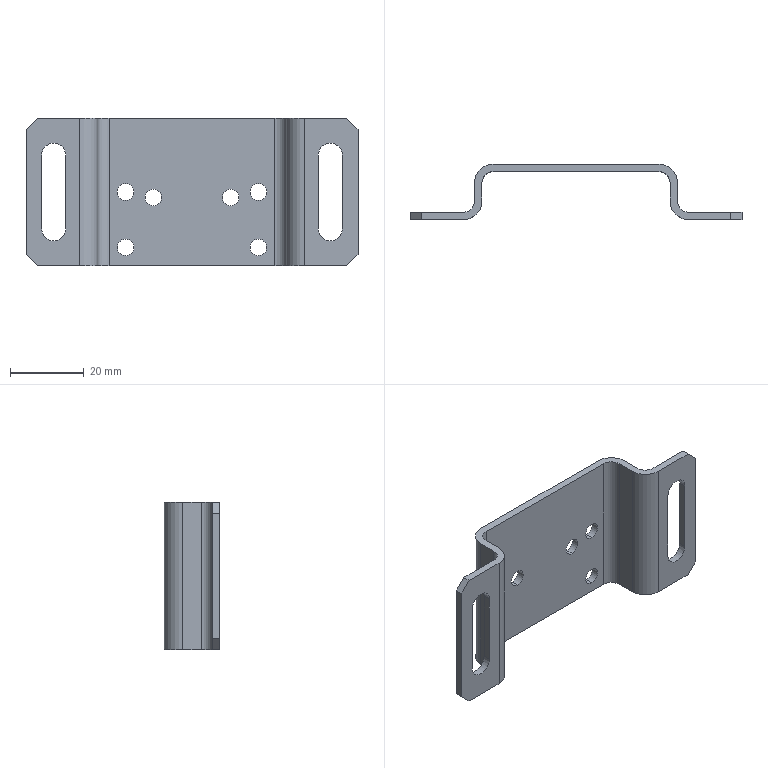Part | SolidWorks | features ICE 2, Chamfer 1, Extrusion 1 | 1 solid | 48 faces | box 90 x 15 x 40 mm | volume 7851 mm3 | cylinder 26 | plane 22 | commonest cylinder face diameters 4.5 x12 6.5 x6 6 x4 10 x4
STEP:
#1=CARTESIAN_POINT('',(27.,11.,2.75));
#2=VERTEX_POINT('',#1);
#3=CARTESIAN_POINT('',(27.,11.,7.25));
#4=VERTEX_POINT('',#3);
#5=CARTESIAN_POINT('',(27.,11.,5.));
#6=DIRECTION('',(0.,1.,0.));
#7=DIRECTION('',(0.,0.,1.));
#8=AXIS2_PLACEMENT_3D('',#5,#6,#7);
#9=CIRCLE('',#8,2.25);
#10=EDGE_CURVE('',#2,#4,#9,.T.);
#11=ORIENTED_EDGE('',*,*,#10,.F.);
#12=CARTESIAN_POINT('',(27.,13.,2.75));
#13=VERTEX_POINT('',#12);
#14=CARTESIAN_POINT('',(27.,-27.,2.75));
#15=DIRECTION('',(0.,1.,0.));
#16=VECTOR('',#15,1000.);
#17=LINE('',#14,#16);
#18=EDGE_CURVE('',#2,#13,#17,.T.);
#19=ORIENTED_EDGE('',*,*,#18,.T.);
#20=CARTESIAN_POINT('',(27.,13.,7.25));
#21=VERTEX_POINT('',#20);
#22=CARTESIAN_POINT('',(27.,13.,5.));
#23=DIRECTION('',(0.,1.,0.));
#24=DIRECTION('',(0.,0.,1.));
#25=AXIS2_PLACEMENT_3D('',#22,#23,#24);
#26=CIRCLE('',#25,2.25);
#27=EDGE_CURVE('',#13,#21,#26,.T.);
#28=ORIENTED_EDGE('',*,*,#27,.T.);
#29=CARTESIAN_POINT('',(27.,-27.,7.25));
#30=DIRECTION('',(0.,1.,0.));
#31=VECTOR('',#30,1000.);
#32=LINE('',#29,#31);
#33=EDGE_CURVE('',#4,#21,#32,.T.);
#34=ORIENTED_EDGE('',*,*,#33,.F.);
#35=EDGE_LOOP('',(#11,#19,#28,#34));
#36=FACE_OUTER_BOUND('',#35,.T.);
#37=CARTESIAN_POINT('',(27.,-27.,5.));
#38=DIRECTION('',(0.,1.,0.));
#39=DIRECTION('',(0.,0.,1.));
#40=AXIS2_PLACEMENT_3D('',#37,#38,#39);
#41=CYLINDRICAL_SURFACE('',#40,2.25);
#42=ADVANCED_FACE('',(#36),#41,.F.);
#43=CARTESIAN_POINT('',(63.,11.,17.75));
#44=VERTEX_POINT('',#43);
#45=CARTESIAN_POINT('',(63.,11.,22.25));
#46=VERTEX_POINT('',#45);
#47=CARTESIAN_POINT('',(63.,11.,20.));
#48=DIRECTION('',(0.,1.,0.));
#49=DIRECTION('',(0.,0.,1.));
#50=AXIS2_PLACEMENT_3D('',#47,#48,#49);
#51=CIRCLE('',#50,2.25);
#52=EDGE_CURVE('',#44,#46,#51,.T.);
#53=ORIENTED_EDGE('',*,*,#52,.F.);
#54=CARTESIAN_POINT('',(63.,13.,17.75));
#55=VERTEX_POINT('',#54);
#56=CARTESIAN_POINT('',(63.,-27.,17.75));
#57=DIRECTION('',(0.,1.,0.));
#58=VECTOR('',#57,1000.);
#59=LINE('',#56,#58);
#60=EDGE_CURVE('',#44,#55,#59,.T.);
#61=ORIENTED_EDGE('',*,*,#60,.T.);
#62=CARTESIAN_POINT('',(63.,13.,22.25));
#63=VERTEX_POINT('',#62);
#64=CARTESIAN_POINT('',(63.,13.,20.));
#65=DIRECTION('',(0.,1.,0.));
#66=DIRECTION('',(0.,0.,1.));
#67=AXIS2_PLACEMENT_3D('',#64,#65,#66);
#68=CIRCLE('',#67,2.25);
#69=EDGE_CURVE('',#55,#63,#68,.T.);
#70=ORIENTED_EDGE('',*,*,#69,.T.);
#71=CARTESIAN_POINT('',(63.,-27.,22.25));
#72=DIRECTION('',(0.,1.,0.));
#73=VECTOR('',#72,1000.);
#74=LINE('',#71,#73);
#75=EDGE_CURVE('',#46,#63,#74,.T.);
#76=ORIENTED_EDGE('',*,*,#75,.F.);
#77=EDGE_LOOP('',(#53,#61,#70,#76));
#78=FACE_OUTER_BOUND('',#77,.T.);
#79=CARTESIAN_POINT('',(63.,-27.,20.));
#80=DIRECTION('',(0.,1.,0.));
#81=DIRECTION('',(0.,0.,1.));
#82=AXIS2_PLACEMENT_3D('',#79,#80,#81);
#83=CYLINDRICAL_SURFACE('',#82,2.25);
#84=ADVANCED_FACE('',(#78),#83,.F.);
#85=CARTESIAN_POINT('',(55.5,11.,16.25));
#86=VERTEX_POINT('',#85);
#87=CARTESIAN_POINT('',(55.5,11.,20.75));
#88=VERTEX_POINT('',#87);
#89=CARTESIAN_POINT('',(55.5,11.,18.5));
#90=DIRECTION('',(0.,1.,0.));
#91=DIRECTION('',(0.,0.,1.));
#92=AXIS2_PLACEMENT_3D('',#89,#90,#91);
#93=CIRCLE('',#92,2.25);
#94=EDGE_CURVE('',#86,#88,#93,.T.);
#95=ORIENTED_EDGE('',*,*,#94,.F.);
#96=CARTESIAN_POINT('',(55.5,13.,16.25));
#97=VERTEX_POINT('',#96);
#98=CARTESIAN_POINT('',(55.5,-27.,16.25));
#99=DIRECTION('',(0.,1.,0.));
#100=VECTOR('',#99,1000.);
#101=LINE('',#98,#100);
#102=EDGE_CURVE('',#86,#97,#101,.T.);
#103=ORIENTED_EDGE('',*,*,#102,.T.);
#104=CARTESIAN_POINT('',(55.5,13.,20.75));
#105=VERTEX_POINT('',#104);
#106=CARTESIAN_POINT('',(55.5,13.,18.5));
#107=DIRECTION('',(0.,1.,0.));
#108=DIRECTION('',(0.,0.,1.));
#109=AXIS2_PLACEMENT_3D('',#106,#107,#108);
#110=CIRCLE('',#109,2.25);
#111=EDGE_CURVE('',#97,#105,#110,.T.);
#112=ORIENTED_EDGE('',*,*,#111,.T.);
#113=CARTESIAN_POINT('',(55.5,-27.,20.75));
#114=DIRECTION('',(0.,1.,0.));
#115=VECTOR('',#114,1000.);
#116=LINE('',#113,#115);
#117=EDGE_CURVE('',#88,#105,#116,.T.);
#118=ORIENTED_EDGE('',*,*,#117,.F.);
#119=EDGE_LOOP('',(#95,#103,#112,#118));
#120=FACE_OUTER_BOUND('',#119,.T.);
#121=CARTESIAN_POINT('',(55.5,-27.,18.5));
#122=DIRECTION('',(0.,1.,0.));
#123=DIRECTION('',(0.,0.,1.));
#124=AXIS2_PLACEMENT_3D('',#121,#122,#123);
#125=CYLINDRICAL_SURFACE('',#124,2.25);
#126=ADVANCED_FACE('',(#120),#125,.F.);
#127=CARTESIAN_POINT('',(27.,11.,17.75));
#128=VERTEX_POINT('',#127);
#129=CARTESIAN_POINT('',(27.,11.,22.25));
#130=VERTEX_POINT('',#129);
#131=CARTESIAN_POINT('',(27.,11.,20.));
#132=DIRECTION('',(0.,1.,0.));
#133=DIRECTION('',(0.,0.,1.));
#134=AXIS2_PLACEMENT_3D('',#131,#132,#133);
#135=CIRCLE('',#134,2.25);
#136=EDGE_CURVE('',#128,#130,#135,.T.);
#137=ORIENTED_EDGE('',*,*,#136,.F.);
#138=CARTESIAN_POINT('',(27.,13.,17.75));
#139=VERTEX_POINT('',#138);
#140=CARTESIAN_POINT('',(27.,-27.,17.75));
#141=DIRECTION('',(0.,1.,0.));
#142=VECTOR('',#141,1000.);
#143=LINE('',#140,#142);
#144=EDGE_CURVE('',#128,#139,#143,.T.);
#145=ORIENTED_EDGE('',*,*,#144,.T.);
#146=CARTESIAN_POINT('',(27.,13.,22.25));
#147=VERTEX_POINT('',#146);
#148=CARTESIAN_POINT('',(27.,13.,20.));
#149=DIRECTION('',(0.,1.,0.));
#150=DIRECTION('',(0.,0.,1.));
#151=AXIS2_PLACEMENT_3D('',#148,#149,#150);
#152=CIRCLE('',#151,2.25);
#153=EDGE_CURVE('',#139,#147,#152,.T.);
#154=ORIENTED_EDGE('',*,*,#153,.T.);
#155=CARTESIAN_POINT('',(27.,-27.,22.25));
#156=DIRECTION('',(0.,1.,0.));
#157=VECTOR('',#156,1000.);
#158=LINE('',#155,#157);
#159=EDGE_CURVE('',#130,#147,#158,.T.);
#160=ORIENTED_EDGE('',*,*,#159,.F.);
#161=EDGE_LOOP('',(#137,#145,#154,#160));
#162=FACE_OUTER_BOUND('',#161,.T.);
#163=CARTESIAN_POINT('',(27.,-27.,20.));
#164=DIRECTION('',(0.,1.,0.));
#165=DIRECTION('',(0.,0.,1.));
#166=AXIS2_PLACEMENT_3D('',#163,#164,#165);
#167=CYLINDRICAL_SURFACE('',#166,2.25);
#168=ADVANCED_FACE('',(#162),#167,.F.);
#169=CARTESIAN_POINT('',(63.,11.,2.75));
#170=VERTEX_POINT('',#169);
#171=CARTESIAN_POINT('',(63.,11.,7.25));
#172=VERTEX_POINT('',#171);
#173=CARTESIAN_POINT('',(63.,11.,5.));
#174=DIRECTION('',(0.,1.,0.));
#175=DIRECTION('',(0.,0.,1.));
#176=AXIS2_PLACEMENT_3D('',#173,#174,#175);
#177=CIRCLE('',#176,2.25);
#178=EDGE_CURVE('',#170,#172,#177,.T.);
#179=ORIENTED_EDGE('',*,*,#178,.F.);
#180=CARTESIAN_POINT('',(63.,13.,2.75));
#181=VERTEX_POINT('',#180);
#182=CARTESIAN_POINT('',(63.,-27.,2.75));
#183=DIRECTION('',(0.,1.,0.));
#184=VECTOR('',#183,1000.);
#185=LINE('',#182,#184);
#186=EDGE_CURVE('',#170,#181,#185,.T.);
#187=ORIENTED_EDGE('',*,*,#186,.T.);
#188=CARTESIAN_POINT('',(63.,13.,7.25));
#189=VERTEX_POINT('',#188);
#190=CARTESIAN_POINT('',(63.,13.,5.));
#191=DIRECTION('',(0.,1.,0.));
#192=DIRECTION('',(0.,0.,1.));
#193=AXIS2_PLACEMENT_3D('',#190,#191,#192);
#194=CIRCLE('',#193,2.25);
#195=EDGE_CURVE('',#181,#189,#194,.T.);
#196=ORIENTED_EDGE('',*,*,#195,.T.);
#197=CARTESIAN_POINT('',(63.,-27.,7.25));
#198=DIRECTION('',(0.,1.,0.));
#199=VECTOR('',#198,1000.);
#200=LINE('',#197,#199);
#201=EDGE_CURVE('',#172,#189,#200,.T.);
#202=ORIENTED_EDGE('',*,*,#201,.F.);
#203=EDGE_LOOP('',(#179,#187,#196,#202));
#204=FACE_OUTER_BOUND('',#203,.T.);
#205=CARTESIAN_POINT('',(63.,-27.,5.));
#206=DIRECTION('',(0.,1.,0.));
#207=DIRECTION('',(0.,0.,1.));
#208=AXIS2_PLACEMENT_3D('',#205,#206,#207);
#209=CYLINDRICAL_SURFACE('',#208,2.25);
#210=ADVANCED_FACE('',(#204),#209,.F.);
#211=CARTESIAN_POINT('',(34.5,11.,16.25));
#212=VERTEX_POINT('',#211);
#213=CARTESIAN_POINT('',(34.5,11.,20.75));
#214=VERTEX_POINT('',#213);
#215=CARTESIAN_POINT('',(34.5,11.,18.5));
#216=DIRECTION('',(0.,1.,0.));
#217=DIRECTION('',(0.,0.,1.));
#218=AXIS2_PLACEMENT_3D('',#215,#216,#217);
#219=CIRCLE('',#218,2.25);
#220=EDGE_CURVE('',#212,#214,#219,.T.);
#221=ORIENTED_EDGE('',*,*,#220,.F.);
#222=CARTESIAN_POINT('',(34.5,13.,16.25));
#223=VERTEX_POINT('',#222);
#224=CARTESIAN_POINT('',(34.5,-27.,16.25));
#225=DIRECTION('',(0.,1.,0.));
#226=VECTOR('',#225,1000.);
#227=LINE('',#224,#226);
#228=EDGE_CURVE('',#212,#223,#227,.T.);
#229=ORIENTED_EDGE('',*,*,#228,.T.);
#230=CARTESIAN_POINT('',(34.5,13.,20.75));
#231=VERTEX_POINT('',#230);
#232=CARTESIAN_POINT('',(34.5,13.,18.5));
#233=DIRECTION('',(0.,1.,0.));
#234=DIRECTION('',(0.,0.,1.));
#235=AXIS2_PLACEMENT_3D('',#232,#233,#234);
#236=CIRCLE('',#235,2.25);
#237=EDGE_CURVE('',#223,#231,#236,.T.);
#238=ORIENTED_EDGE('',*,*,#237,.T.);
#239=CARTESIAN_POINT('',(34.5,-27.,20.75));
#240=DIRECTION('',(0.,1.,0.));
#241=VECTOR('',#240,1000.);
#242=LINE('',#239,#241);
#243=EDGE_CURVE('',#214,#231,#242,.T.);
#244=ORIENTED_EDGE('',*,*,#243,.F.);
#245=EDGE_LOOP('',(#221,#229,#238,#244));
#246=FACE_OUTER_BOUND('',#245,.T.);
#247=CARTESIAN_POINT('',(34.5,-27.,18.5));
#248=DIRECTION('',(0.,1.,0.));
#249=DIRECTION('',(0.,0.,1.));
#250=AXIS2_PLACEMENT_3D('',#247,#248,#249);
#251=CYLINDRICAL_SURFACE('',#250,2.25);
#252=ADVANCED_FACE('',(#246),#251,.F.);
#253=CARTESIAN_POINT('',(7.5,-2.,33.25));
#254=VERTEX_POINT('',#253);
#255=CARTESIAN_POINT('',(10.75,-2.,30.));
#256=VERTEX_POINT('',#255);
#257=CARTESIAN_POINT('',(7.5,-2.,30.));
#258=DIRECTION('',(0.,1.,0.));
#259=DIRECTION('',(0.,0.,1.));
#260=AXIS2_PLACEMENT_3D('',#257,#258,#259);
#261=CIRCLE('',#260,3.25);
#262=EDGE_CURVE('',#254,#256,#261,.T.);
#263=ORIENTED_EDGE('',*,*,#262,.F.);
#264=CARTESIAN_POINT('',(7.5,0.,33.25));
#265=VERTEX_POINT('',#264);
#266=CARTESIAN_POINT('',(7.5,-40.,33.25));
#267=DIRECTION('',(0.,1.,0.));
#268=VECTOR('',#267,1000.);
#269=LINE('',#266,#268);
#270=EDGE_CURVE('',#254,#265,#269,.T.);
#271=ORIENTED_EDGE('',*,*,#270,.T.);
#272=CARTESIAN_POINT('',(10.75,0.,30.));
#273=VERTEX_POINT('',#272);
#274=CARTESIAN_POINT('',(7.5,0.,30.));
#275=DIRECTION('',(0.,1.,0.));
#276=DIRECTION('',(0.,0.,1.));
#277=AXIS2_PLACEMENT_3D('',#274,#275,#276);
#278=CIRCLE('',#277,3.25);
#279=EDGE_CURVE('',#265,#273,#278,.T.);
#280=ORIENTED_EDGE('',*,*,#279,.T.);
#281=CARTESIAN_POINT('',(10.75,-40.,30.));
#282=DIRECTION('',(0.,1.,0.));
#283=VECTOR('',#282,1000.);
#284=LINE('',#281,#283);
#285=EDGE_CURVE('',#256,#273,#284,.T.);
#286=ORIENTED_EDGE('',*,*,#285,.F.);
#287=EDGE_LOOP('',(#263,#271,#280,#286));
#288=FACE_OUTER_BOUND('',#287,.T.);
#289=CARTESIAN_POINT('',(7.5,-40.,30.));
#290=DIRECTION('',(0.,1.,0.));
#291=DIRECTION('',(0.,0.,1.));
#292=AXIS2_PLACEMENT_3D('',#289,#290,#291);
#293=CYLINDRICAL_SURFACE('',#292,3.25);
#294=ADVANCED_FACE('',(#288),#293,.F.);
#295=CARTESIAN_POINT('',(85.75,-2.,30.));
#296=VERTEX_POINT('',#295);
#297=CARTESIAN_POINT('',(82.5,-2.,33.25));
#298=VERTEX_POINT('',#297);
#299=CARTESIAN_POINT('',(82.5,-2.,30.));
#300=DIRECTION('',(0.,-1.,0.));
#301=DIRECTION('',(-1.,0.,0.));
#302=AXIS2_PLACEMENT_3D('',#299,#300,#301);
#303=CIRCLE('',#302,3.25);
#304=EDGE_CURVE('',#296,#298,#303,.T.);
#305=ORIENTED_EDGE('',*,*,#304,.T.);
#306=CARTESIAN_POINT('',(82.5,0.,33.25));
#307=VERTEX_POINT('',#306);
#308=CARTESIAN_POINT('',(82.5,-40.,33.25));
#309=DIRECTION('',(0.,1.,0.));
#310=VECTOR('',#309,1000.);
#311=LINE('',#308,#310);
#312=EDGE_CURVE('',#298,#307,#311,.T.);
#313=ORIENTED_EDGE('',*,*,#312,.T.);
#314=CARTESIAN_POINT('',(85.75,0.,30.));
#315=VERTEX_POINT('',#314);
#316=CARTESIAN_POINT('',(82.5,0.,30.));
#317=DIRECTION('',(0.,-1.,0.));
#318=DIRECTION('',(0.,0.,1.));
#319=AXIS2_PLACEMENT_3D('',#316,#317,#318);
#320=CIRCLE('',#319,3.25);
#321=EDGE_CURVE('',#315,#307,#320,.T.);
#322=ORIENTED_EDGE('',*,*,#321,.F.);
#323=CARTESIAN_POINT('',(85.75,-40.,30.));
#324=DIRECTION('',(0.,1.,0.));
#325=VECTOR('',#324,1000.);
#326=LINE('',#323,#325);
#327=EDGE_CURVE('',#296,#315,#326,.T.);
#328=ORIENTED_EDGE('',*,*,#327,.F.);
#329=EDGE_LOOP('',(#305,#313,#322,#328));
#330=FACE_OUTER_BOUND('',#329,.T.);
#331=CARTESIAN_POINT('',(82.5,-40.,30.));
#332=DIRECTION('',(0.,1.,0.));
#333=DIRECTION('',(0.,0.,1.));
#334=AXIS2_PLACEMENT_3D('',#331,#332,#333);
#335=CYLINDRICAL_SURFACE('',#334,3.25);
#336=ADVANCED_FACE('',(#330),#335,.F.);
#337=CARTESIAN_POINT('',(90.,0.,37.));
#338=VERTEX_POINT('',#337);
#339=CARTESIAN_POINT('',(90.,0.,3.));
#340=VERTEX_POINT('',#339);
#341=CARTESIAN_POINT('',(90.,0.,40.));
#342=DIRECTION('',(0.,0.,-1.));
#343=VECTOR('',#342,1000.);
#344=LINE('',#341,#343);
#345=EDGE_CURVE('',#338,#340,#344,.T.);
#346=ORIENTED_EDGE('',*,*,#345,.T.);
#347=CARTESIAN_POINT('',(87.,0.,0.));
#348=VERTEX_POINT('',#347);
#349=CARTESIAN_POINT('',(101.25,0.,14.25));
#350=DIRECTION('',(-0.7071,0.,-0.7071));
#351=VECTOR('',#350,1000.);
#352=LINE('',#349,#351);
#353=EDGE_CURVE('',#340,#348,#352,.T.);
#354=ORIENTED_EDGE('',*,*,#353,.T.);
#355=CARTESIAN_POINT('',(75.5,0.,0.));
#356=VERTEX_POINT('',#355);
#357=CARTESIAN_POINT('',(75.5,0.,0.));
#358=DIRECTION('',(1.,0.,0.));
#359=VECTOR('',#358,1000.);
#360=LINE('',#357,#359);
#361=EDGE_CURVE('',#356,#348,#360,.T.);
#362=ORIENTED_EDGE('',*,*,#361,.F.);
#363=CARTESIAN_POINT('',(75.5,0.,40.));
#364=VERTEX_POINT('',#363);
#365=CARTESIAN_POINT('',(75.5,0.,40.));
#366=DIRECTION('',(0.,0.,-1.));
#367=VECTOR('',#366,1000.);
#368=LINE('',#365,#367);
#369=EDGE_CURVE('',#364,#356,#368,.T.);
#370=ORIENTED_EDGE('',*,*,#369,.F.);
#371=CARTESIAN_POINT('',(87.,0.,40.));
#372=VERTEX_POINT('',#371);
#373=CARTESIAN_POINT('',(75.5,0.,40.));
#374=DIRECTION('',(1.,0.,0.));
#375=VECTOR('',#374,1000.);
#376=LINE('',#373,#375);
#377=EDGE_CURVE('',#364,#372,#376,.T.);
#378=ORIENTED_EDGE('',*,*,#377,.T.);
#379=CARTESIAN_POINT('',(81.25,0.,45.75));
#380=DIRECTION('',(0.7071,0.,-0.7071));
#381=VECTOR('',#380,1000.);
#382=LINE('',#379,#381);
#383=EDGE_CURVE('',#372,#338,#382,.T.);
#384=ORIENTED_EDGE('',*,*,#383,.T.);
#385=EDGE_LOOP('',(#346,#354,#362,#370,#378,#384));
#386=FACE_OUTER_BOUND('',#385,.T.);
#387=CARTESIAN_POINT('',(85.75,0.,10.));
#388=VERTEX_POINT('',#387);
#389=CARTESIAN_POINT('',(85.75,0.,0.));
#390=DIRECTION('',(0.,0.,1.));
#391=VECTOR('',#390,1000.);
#392=LINE('',#389,#391);
#393=EDGE_CURVE('',#388,#315,#392,.T.);
#394=ORIENTED_EDGE('',*,*,#393,.T.);
#395=ORIENTED_EDGE('',*,*,#321,.T.);
#396=CARTESIAN_POINT('',(79.25,0.,30.));
#397=VERTEX_POINT('',#396);
#398=CARTESIAN_POINT('',(82.5,0.,30.));
#399=DIRECTION('',(0.,-1.,0.));
#400=DIRECTION('',(0.,0.,1.));
#401=AXIS2_PLACEMENT_3D('',#398,#399,#400);
#402=CIRCLE('',#401,3.25);
#403=EDGE_CURVE('',#307,#397,#402,.T.);
#404=ORIENTED_EDGE('',*,*,#403,.T.);
#405=CARTESIAN_POINT('',(79.25,0.,10.));
#406=VERTEX_POINT('',#405);
#407=CARTESIAN_POINT('',(79.25,0.,0.));
#408=DIRECTION('',(0.,0.,1.));
#409=VECTOR('',#408,1000.);
#410=LINE('',#407,#409);
#411=EDGE_CURVE('',#406,#397,#410,.T.);
#412=ORIENTED_EDGE('',*,*,#411,.F.);
#413=CARTESIAN_POINT('',(82.5,0.,10.));
#414=DIRECTION('',(0.,-1.,0.));
#415=DIRECTION('',(0.,0.,1.));
#416=AXIS2_PLACEMENT_3D('',#413,#414,#415);
#417=CIRCLE('',#416,3.25);
#418=EDGE_CURVE('',#406,#388,#417,.T.);
#419=ORIENTED_EDGE('',*,*,#418,.T.);
#420=EDGE_LOOP('',(#394,#395,#404,#412,#419));
#421=FACE_BOUND('',#420,.T.);
#422=CARTESIAN_POINT('',(75.5,0.,40.));
#423=DIRECTION('',(0.,1.,0.));
#424=DIRECTION('',(0.,0.,1.));
#425=AXIS2_PLACEMENT_3D('',#422,#423,#424);
#426=PLANE('',#425);
#427=ADVANCED_FACE('',(#386,#421),#426,.T.);
#428=CARTESIAN_POINT('',(75.5,-2.,0.));
#429=VERTEX_POINT('',#428);
#430=CARTESIAN_POINT('',(87.,-2.,0.));
#431=VERTEX_POINT('',#430);
#432=CARTESIAN_POINT('',(75.5,-2.,0.));
#433=DIRECTION('',(1.,0.,0.));
#434=VECTOR('',#433,1000.);
#435=LINE('',#432,#434);
#436=EDGE_CURVE('',#429,#431,#435,.T.);
#437=ORIENTED_EDGE('',*,*,#436,.T.);
#438=CARTESIAN_POINT('',(90.,-2.,3.));
#439=VERTEX_POINT('',#438);
#440=CARTESIAN_POINT('',(87.,-2.,0.));
#441=DIRECTION('',(0.7071,0.,0.7071));
#442=VECTOR('',#441,1000.);
#443=LINE('',#440,#442);
#444=EDGE_CURVE('',#431,#439,#443,.T.);
#445=ORIENTED_EDGE('',*,*,#444,.T.);
#446=CARTESIAN_POINT('',(90.,-2.,37.));
#447=VERTEX_POINT('',#446);
#448=CARTESIAN_POINT('',(90.,-2.,40.));
#449=DIRECTION('',(0.,0.,-1.));
#450=VECTOR('',#449,1000.);
#451=LINE('',#448,#450);
#452=EDGE_CURVE('',#447,#439,#451,.T.);
#453=ORIENTED_EDGE('',*,*,#452,.F.);
#454=CARTESIAN_POINT('',(87.,-2.,40.));
#455=VERTEX_POINT('',#454);
#456=CARTESIAN_POINT('',(90.,-2.,37.));
#457=DIRECTION('',(-0.7071,0.,0.7071));
#458=VECTOR('',#457,1000.);
#459=LINE('',#456,#458);
#460=EDGE_CURVE('',#447,#455,#459,.T.);
#461=ORIENTED_EDGE('',*,*,#460,.T.);
#462=CARTESIAN_POINT('',(75.5,-2.,40.));
#463=VERTEX_POINT('',#462);
#464=CARTESIAN_POINT('',(75.5,-2.,40.));
#465=DIRECTION('',(1.,0.,0.));
#466=VECTOR('',#465,1000.);
#467=LINE('',#464,#466);
#468=EDGE_CURVE('',#463,#455,#467,.T.);
#469=ORIENTED_EDGE('',*,*,#468,.F.);
#470=CARTESIAN_POINT('',(75.5,-2.,40.));
#471=DIRECTION('',(0.,0.,-1.));
#472=VECTOR('',#471,1000.);
#473=LINE('',#470,#472);
#474=EDGE_CURVE('',#463,#429,#473,.T.);
#475=ORIENTED_EDGE('',*,*,#474,.T.);
#476=EDGE_LOOP('',(#437,#445,#453,#461,#469,#475));
#477=FACE_OUTER_BOUND('',#476,.T.);
#478=ORIENTED_EDGE('',*,*,#304,.F.);
#479=CARTESIAN_POINT('',(85.75,-2.,10.));
#480=VERTEX_POINT('',#479);
#481=CARTESIAN_POINT('',(85.75,-2.,40.));
#482=DIRECTION('',(0.,0.,1.));
#483=VECTOR('',#482,1000.);
#484=LINE('',#481,#483);
#485=EDGE_CURVE('',#480,#296,#484,.T.);
#486=ORIENTED_EDGE('',*,*,#485,.F.);
#487=CARTESIAN_POINT('',(79.25,-2.,10.));
#488=VERTEX_POINT('',#487);
#489=CARTESIAN_POINT('',(82.5,-2.,10.));
#490=DIRECTION('',(0.,-1.,0.));
#491=DIRECTION('',(-1.,0.,0.));
#492=AXIS2_PLACEMENT_3D('',#489,#490,#491);
#493=CIRCLE('',#492,3.25);
#494=EDGE_CURVE('',#488,#480,#493,.T.);
#495=ORIENTED_EDGE('',*,*,#494,.F.);
#496=CARTESIAN_POINT('',(79.25,-2.,30.));
#497=VERTEX_POINT('',#496);
#498=CARTESIAN_POINT('',(79.25,-2.,40.));
#499=DIRECTION('',(0.,0.,1.));
#500=VECTOR('',#499,1000.);
#501=LINE('',#498,#500);
#502=EDGE_CURVE('',#488,#497,#501,.T.);
#503=ORIENTED_EDGE('',*,*,#502,.T.);
#504=CARTESIAN_POINT('',(82.5,-2.,30.));
#505=DIRECTION('',(0.,-1.,0.));
#506=DIRECTION('',(-1.,0.,0.));
#507=AXIS2_PLACEMENT_3D('',#504,#505,#506);
#508=CIRCLE('',#507,3.25);
#509=EDGE_CURVE('',#298,#497,#508,.T.);
#510=ORIENTED_EDGE('',*,*,#509,.F.);
#511=EDGE_LOOP('',(#478,#486,#495,#503,#510));
#512=FACE_BOUND('',#511,.T.);
#513=CARTESIAN_POINT('',(75.5,-2.,40.));
#514=DIRECTION('',(0.,1.,0.));
#515=DIRECTION('',(-1.,0.,0.));
#516=AXIS2_PLACEMENT_3D('',#513,#514,#515);
#517=PLANE('',#516);
#518=ADVANCED_FACE('',(#477,#512),#517,.F.);
#519=CARTESIAN_POINT('',(72.5,3.,0.));
#520=VERTEX_POINT('',#519);
#521=CARTESIAN_POINT('',(75.5,3.,0.));
#522=DIRECTION('',(0.,0.,1.));
#523=DIRECTION('',(1.,0.,0.));
#524=AXIS2_PLACEMENT_3D('',#521,#522,#523);
#525=CIRCLE('',#524,3.);
#526=EDGE_CURVE('',#520,#356,#525,.T.);
#527=ORIENTED_EDGE('',*,*,#526,.F.);
#528=CARTESIAN_POINT('',(72.5,3.,40.));
#529=VERTEX_POINT('',#528);
#530=CARTESIAN_POINT('',(72.5,3.,40.));
#531=DIRECTION('',(0.,0.,-1.));
#532=VECTOR('',#531,1000.);
#533=LINE('',#530,#532);
#534=EDGE_CURVE('',#529,#520,#533,.T.);
#535=ORIENTED_EDGE('',*,*,#534,.F.);
#536=CARTESIAN_POINT('',(75.5,3.,40.));
#537=DIRECTION('',(0.,0.,1.));
#538=DIRECTION('',(1.,0.,0.));
#539=AXIS2_PLACEMENT_3D('',#536,#537,#538);
#540=CIRCLE('',#539,3.);
#541=EDGE_CURVE('',#529,#364,#540,.T.);
#542=ORIENTED_EDGE('',*,*,#541,.T.);
#543=ORIENTED_EDGE('',*,*,#369,.T.);
#544=EDGE_LOOP('',(#527,#535,#542,#543));
#545=FACE_OUTER_BOUND('',#544,.T.);
#546=CARTESIAN_POINT('',(75.5,3.,40.));
#547=DIRECTION('',(0.,0.,-1.));
#548=DIRECTION('',(-1.,0.,0.));
#549=AXIS2_PLACEMENT_3D('',#546,#547,#548);
#550=CYLINDRICAL_SURFACE('',#549,3.);
#551=ADVANCED_FACE('',(#545),#550,.F.);
#552=CARTESIAN_POINT('',(72.5,8.,0.));
#553=VERTEX_POINT('',#552);
#554=CARTESIAN_POINT('',(72.5,8.,0.));
#555=DIRECTION('',(0.,-1.,0.));
#556=VECTOR('',#555,1000.);
#557=LINE('',#554,#556);
#558=EDGE_CURVE('',#553,#520,#557,.T.);
#559=ORIENTED_EDGE('',*,*,#558,.F.);
#560=CARTESIAN_POINT('',(72.5,8.,40.));
#561=VERTEX_POINT('',#560);
#562=CARTESIAN_POINT('',(72.5,8.,40.));
#563=DIRECTION('',(0.,0.,-1.));
#564=VECTOR('',#563,1000.);
#565=LINE('',#562,#564);
#566=EDGE_CURVE('',#561,#553,#565,.T.);
#567=ORIENTED_EDGE('',*,*,#566,.F.);
#568=CARTESIAN_POINT('',(72.5,8.,40.));
#569=DIRECTION('',(0.,-1.,0.));
#570=VECTOR('',#569,1000.);
#571=LINE('',#568,#570);
#572=EDGE_CURVE('',#561,#529,#571,.T.);
#573=ORIENTED_EDGE('',*,*,#572,.T.);
#574=ORIENTED_EDGE('',*,*,#534,.T.);
#575=EDGE_LOOP('',(#559,#567,#573,#574));
#576=FACE_OUTER_BOUND('',#575,.T.);
#577=CARTESIAN_POINT('',(72.5,8.,40.));
#578=DIRECTION('',(1.,0.,0.));
#579=DIRECTION('',(0.,0.,-1.));
#580=AXIS2_PLACEMENT_3D('',#577,#578,#579);
#581=PLANE('',#580);
#582=ADVANCED_FACE('',(#576),#581,.T.);
#583=CARTESIAN_POINT('',(67.5,13.,0.));
#584=VERTEX_POINT('',#583);
#585=CARTESIAN_POINT('',(67.5,8.,0.));
#586=DIRECTION('',(0.,0.,-1.));
#587=DIRECTION('',(-1.,0.,0.));
#588=AXIS2_PLACEMENT_3D('',#585,#586,#587);
#589=CIRCLE('',#588,5.);
#590=EDGE_CURVE('',#584,#553,#589,.T.);
#591=ORIENTED_EDGE('',*,*,#590,.F.);
#592=CARTESIAN_POINT('',(67.5,13.,40.));
#593=VERTEX_POINT('',#592);
#594=CARTESIAN_POINT('',(67.5,13.,40.));
#595=DIRECTION('',(0.,0.,-1.));
#596=VECTOR('',#595,1000.);
#597=LINE('',#594,#596);
#598=EDGE_CURVE('',#593,#584,#597,.T.);
#599=ORIENTED_EDGE('',*,*,#598,.F.);
#600=CARTESIAN_POINT('',(67.5,8.,40.));
#601=DIRECTION('',(0.,0.,-1.));
#602=DIRECTION('',(-1.,0.,0.));
#603=AXIS2_PLACEMENT_3D('',#600,#601,#602);
#604=CIRCLE('',#603,5.);
#605=EDGE_CURVE('',#593,#561,#604,.T.);
#606=ORIENTED_EDGE('',*,*,#605,.T.);
#607=ORIENTED_EDGE('',*,*,#566,.T.);
#608=EDGE_LOOP('',(#591,#599,#606,#607));
#609=FACE_OUTER_BOUND('',#608,.T.);
#610=CARTESIAN_POINT('',(67.5,8.,40.));
#611=DIRECTION('',(0.,0.,-1.));
#612=DIRECTION('',(-1.,0.,0.));
#613=AXIS2_PLACEMENT_3D('',#610,#611,#612);
#614=CYLINDRICAL_SURFACE('',#613,5.);
#615=ADVANCED_FACE('',(#609),#614,.T.);
#616=CARTESIAN_POINT('',(27.,13.,5.));
#617=DIRECTION('',(0.,1.,0.));
#618=DIRECTION('',(0.,0.,1.));
#619=AXIS2_PLACEMENT_3D('',#616,#617,#618);
#620=CIRCLE('',#619,2.25);
#621=EDGE_CURVE('',#21,#13,#620,.T.);
#622=ORIENTED_EDGE('',*,*,#621,.F.);
#623=ORIENTED_EDGE('',*,*,#27,.F.);
#624=EDGE_LOOP('',(#622,#623));
#625=FACE_BOUND('',#624,.T.);
#626=CARTESIAN_POINT('',(63.,13.,20.));
#627=DIRECTION('',(0.,1.,0.));
#628=DIRECTION('',(0.,0.,1.));
#629=AXIS2_PLACEMENT_3D('',#626,#627,#628);
#630=CIRCLE('',#629,2.25);
#631=EDGE_CURVE('',#63,#55,#630,.T.);
#632=ORIENTED_EDGE('',*,*,#631,.F.);
#633=ORIENTED_EDGE('',*,*,#69,.F.);
#634=EDGE_LOOP('',(#632,#633));
#635=FACE_BOUND('',#634,.T.);
#636=CARTESIAN_POINT('',(55.5,13.,18.5));
#637=DIRECTION('',(0.,1.,0.));
#638=DIRECTION('',(0.,0.,1.));
#639=AXIS2_PLACEMENT_3D('',#636,#637,#638);
#640=CIRCLE('',#639,2.25);
#641=EDGE_CURVE('',#105,#97,#640,.T.);
#642=ORIENTED_EDGE('',*,*,#641,.F.);
#643=ORIENTED_EDGE('',*,*,#111,.F.);
#644=EDGE_LOOP('',(#642,#643));
#645=FACE_BOUND('',#644,.T.);
#646=CARTESIAN_POINT('',(27.,13.,20.));
#647=DIRECTION('',(0.,1.,0.));
#648=DIRECTION('',(0.,0.,1.));
#649=AXIS2_PLACEMENT_3D('',#646,#647,#648);
#650=CIRCLE('',#649,2.25);
#651=EDGE_CURVE('',#147,#139,#650,.T.);
#652=ORIENTED_EDGE('',*,*,#651,.F.);
#653=ORIENTED_EDGE('',*,*,#153,.F.);
#654=EDGE_LOOP('',(#652,#653));
#655=FACE_BOUND('',#654,.T.);
#656=CARTESIAN_POINT('',(63.,13.,5.));
#657=DIRECTION('',(0.,1.,0.));
#658=DIRECTION('',(0.,0.,1.));
#659=AXIS2_PLACEMENT_3D('',#656,#657,#658);
#660=CIRCLE('',#659,2.25);
#661=EDGE_CURVE('',#189,#181,#660,.T.);
#662=ORIENTED_EDGE('',*,*,#661,.F.);
#663=ORIENTED_EDGE('',*,*,#195,.F.);
#664=EDGE_LOOP('',(#662,#663));
#665=FACE_BOUND('',#664,.T.);
#666=CARTESIAN_POINT('',(34.5,13.,18.5));
#667=DIRECTION('',(0.,1.,0.));
#668=DIRECTION('',(0.,0.,1.));
#669=AXIS2_PLACEMENT_3D('',#666,#667,#668);
#670=CIRCLE('',#669,2.25);
#671=EDGE_CURVE('',#231,#223,#670,.T.);
#672=ORIENTED_EDGE('',*,*,#671,.F.);
#673=ORIENTED_EDGE('',*,*,#237,.F.);
#674=EDGE_LOOP('',(#672,#673));
#675=FACE_BOUND('',#674,.T.);
#676=CARTESIAN_POINT('',(22.5,13.,0.));
#677=VERTEX_POINT('',#676);
#678=CARTESIAN_POINT('',(22.5,13.,0.));
#679=DIRECTION('',(1.,0.,0.));
#680=VECTOR('',#679,1000.);
#681=LINE('',#678,#680);
#682=EDGE_CURVE('',#677,#584,#681,.T.);
#683=ORIENTED_EDGE('',*,*,#682,.F.);
#684=CARTESIAN_POINT('',(22.5,13.,40.));
#685=VERTEX_POINT('',#684);
#686=CARTESIAN_POINT('',(22.5,13.,40.));
#687=DIRECTION('',(0.,0.,-1.));
#688=VECTOR('',#687,1000.);
#689=LINE('',#686,#688);
#690=EDGE_CURVE('',#685,#677,#689,.T.);
#691=ORIENTED_EDGE('',*,*,#690,.F.);
#692=CARTESIAN_POINT('',(22.5,13.,40.));
#693=DIRECTION('',(1.,0.,0.));
#694=VECTOR('',#693,1000.);
#695=LINE('',#692,#694);
#696=EDGE_CURVE('',#685,#593,#695,.T.);
#697=ORIENTED_EDGE('',*,*,#696,.T.);
#698=ORIENTED_EDGE('',*,*,#598,.T.);
#699=EDGE_LOOP('',(#683,#691,#697,#698));
#700=FACE_OUTER_BOUND('',#699,.T.);
#701=CARTESIAN_POINT('',(22.5,13.,40.));
#702=DIRECTION('',(0.,1.,0.));
#703=DIRECTION('',(0.,0.,1.));
#704=AXIS2_PLACEMENT_3D('',#701,#702,#703);
#705=PLANE('',#704);
#706=ADVANCED_FACE('',(#625,#635,#645,#655,#665,#675,#700),#705,.T.);
#707=CARTESIAN_POINT('',(17.5,8.,0.));
#708=VERTEX_POINT('',#707);
#709=CARTESIAN_POINT('',(22.5,8.,0.));
#710=DIRECTION('',(0.,0.,-1.));
#711=DIRECTION('',(-1.,0.,0.));
#712=AXIS2_PLACEMENT_3D('',#709,#710,#711);
#713=CIRCLE('',#712,5.);
#714=EDGE_CURVE('',#708,#677,#713,.T.);
#715=ORIENTED_EDGE('',*,*,#714,.F.);
#716=CARTESIAN_POINT('',(17.5,8.,40.));
#717=VERTEX_POINT('',#716);
#718=CARTESIAN_POINT('',(17.5,8.,40.));
#719=DIRECTION('',(0.,0.,-1.));
#720=VECTOR('',#719,1000.);
#721=LINE('',#718,#720);
#722=EDGE_CURVE('',#717,#708,#721,.T.);
#723=ORIENTED_EDGE('',*,*,#722,.F.);
#724=CARTESIAN_POINT('',(22.5,8.,40.));
#725=DIRECTION('',(0.,0.,-1.));
#726=DIRECTION('',(-1.,0.,0.));
#727=AXIS2_PLACEMENT_3D('',#724,#725,#726);
#728=CIRCLE('',#727,5.);
#729=EDGE_CURVE('',#717,#685,#728,.T.);
#730=ORIENTED_EDGE('',*,*,#729,.T.);
#731=ORIENTED_EDGE('',*,*,#690,.T.);
#732=EDGE_LOOP('',(#715,#723,#730,#731));
#733=FACE_OUTER_BOUND('',#732,.T.);
#734=CARTESIAN_POINT('',(22.5,8.,40.));
#735=DIRECTION('',(0.,0.,-1.));
#736=DIRECTION('',(-1.,0.,0.));
#737=AXIS2_PLACEMENT_3D('',#734,#735,#736);
#738=CYLINDRICAL_SURFACE('',#737,5.);
#739=ADVANCED_FACE('',(#733),#738,.T.);
#740=CARTESIAN_POINT('',(17.5,3.,0.));
#741=VERTEX_POINT('',#740);
#742=CARTESIAN_POINT('',(17.5,3.,0.));
#743=DIRECTION('',(0.,1.,0.));
#744=VECTOR('',#743,1000.);
#745=LINE('',#742,#744);
#746=EDGE_CURVE('',#741,#708,#745,.T.);
#747=ORIENTED_EDGE('',*,*,#746,.F.);
#748=CARTESIAN_POINT('',(17.5,3.,40.));
#749=VERTEX_POINT('',#748);
#750=CARTESIAN_POINT('',(17.5,3.,40.));
#751=DIRECTION('',(0.,0.,-1.));
#752=VECTOR('',#751,1000.);
#753=LINE('',#750,#752);
#754=EDGE_CURVE('',#749,#741,#753,.T.);
#755=ORIENTED_EDGE('',*,*,#754,.F.);
#756=CARTESIAN_POINT('',(17.5,3.,40.));
#757=DIRECTION('',(0.,1.,0.));
#758=VECTOR('',#757,1000.);
#759=LINE('',#756,#758);
#760=EDGE_CURVE('',#749,#717,#759,.T.);
#761=ORIENTED_EDGE('',*,*,#760,.T.);
#762=ORIENTED_EDGE('',*,*,#722,.T.);
#763=EDGE_LOOP('',(#747,#755,#761,#762));
#764=FACE_OUTER_BOUND('',#763,.T.);
#765=CARTESIAN_POINT('',(17.5,3.,40.));
#766=DIRECTION('',(-1.,0.,0.));
#767=DIRECTION('',(0.,0.,1.));
#768=AXIS2_PLACEMENT_3D('',#765,#766,#767);
#769=PLANE('',#768);
#770=ADVANCED_FACE('',(#764),#769,.T.);
#771=CARTESIAN_POINT('',(14.5,0.,0.));
#772=VERTEX_POINT('',#771);
#773=CARTESIAN_POINT('',(14.5,3.,0.));
#774=DIRECTION('',(0.,0.,1.));
#775=DIRECTION('',(1.,0.,0.));
#776=AXIS2_PLACEMENT_3D('',#773,#774,#775);
#777=CIRCLE('',#776,3.);
#778=EDGE_CURVE('',#772,#741,#777,.T.);
#779=ORIENTED_EDGE('',*,*,#778,.F.);
#780=CARTESIAN_POINT('',(14.5,0.,40.));
#781=VERTEX_POINT('',#780);
#782=CARTESIAN_POINT('',(14.5,0.,40.));
#783=DIRECTION('',(0.,0.,-1.));
#784=VECTOR('',#783,1000.);
#785=LINE('',#782,#784);
#786=EDGE_CURVE('',#781,#772,#785,.T.);
#787=ORIENTED_EDGE('',*,*,#786,.F.);
#788=CARTESIAN_POINT('',(14.5,3.,40.));
#789=DIRECTION('',(0.,0.,1.));
#790=DIRECTION('',(1.,0.,0.));
#791=AXIS2_PLACEMENT_3D('',#788,#789,#790);
#792=CIRCLE('',#791,3.);
#793=EDGE_CURVE('',#781,#749,#792,.T.);
#794=ORIENTED_EDGE('',*,*,#793,.T.);
#795=ORIENTED_EDGE('',*,*,#754,.T.);
#796=EDGE_LOOP('',(#779,#787,#794,#795));
#797=FACE_OUTER_BOUND('',#796,.T.);
#798=CARTESIAN_POINT('',(14.5,3.,40.));
#799=DIRECTION('',(0.,0.,-1.));
#800=DIRECTION('',(-1.,0.,0.));
#801=AXIS2_PLACEMENT_3D('',#798,#799,#800);
#802=CYLINDRICAL_SURFACE('',#801,3.);
#803=ADVANCED_FACE('',(#797),#802,.F.);
#804=CARTESIAN_POINT('',(4.25,0.,10.));
#805=VERTEX_POINT('',#804);
#806=CARTESIAN_POINT('',(4.25,0.,30.));
#807=VERTEX_POINT('',#806);
#808=CARTESIAN_POINT('',(4.25,0.,0.));
#809=DIRECTION('',(0.,0.,1.));
#810=VECTOR('',#809,1000.);
#811=LINE('',#808,#810);
#812=EDGE_CURVE('',#805,#807,#811,.T.);
#813=ORIENTED_EDGE('',*,*,#812,.F.);
#814=CARTESIAN_POINT('',(10.75,0.,10.));
#815=VERTEX_POINT('',#814);
#816=CARTESIAN_POINT('',(7.5,0.,10.));
#817=DIRECTION('',(0.,1.,0.));
#818=DIRECTION('',(0.,0.,1.));
#819=AXIS2_PLACEMENT_3D('',#816,#817,#818);
#820=CIRCLE('',#819,3.25);
#821=EDGE_CURVE('',#815,#805,#820,.T.);
#822=ORIENTED_EDGE('',*,*,#821,.F.);
#823=CARTESIAN_POINT('',(10.75,0.,0.));
#824=DIRECTION('',(0.,0.,1.));
#825=VECTOR('',#824,1000.);
#826=LINE('',#823,#825);
#827=EDGE_CURVE('',#815,#273,#826,.T.);
#828=ORIENTED_EDGE('',*,*,#827,.T.);
#829=ORIENTED_EDGE('',*,*,#279,.F.);
#830=CARTESIAN_POINT('',(7.5,0.,30.));
#831=DIRECTION('',(0.,1.,0.));
#832=DIRECTION('',(0.,0.,1.));
#833=AXIS2_PLACEMENT_3D('',#830,#831,#832);
#834=CIRCLE('',#833,3.25);
#835=EDGE_CURVE('',#807,#265,#834,.T.);
#836=ORIENTED_EDGE('',*,*,#835,.F.);
#837=EDGE_LOOP('',(#813,#822,#828,#829,#836));
#838=FACE_BOUND('',#837,.T.);
#839=CARTESIAN_POINT('',(3.,0.,0.));
#840=VERTEX_POINT('',#839);
#841=CARTESIAN_POINT('',(0.,0.,0.));
#842=DIRECTION('',(1.,0.,0.));
#843=VECTOR('',#842,1000.);
#844=LINE('',#841,#843);
#845=EDGE_CURVE('',#840,#772,#844,.T.);
#846=ORIENTED_EDGE('',*,*,#845,.F.);
#847=CARTESIAN_POINT('',(0.,0.,3.));
#848=VERTEX_POINT('',#847);
#849=CARTESIAN_POINT('',(-18.5,0.,21.5));
#850=DIRECTION('',(-0.7071,0.,0.7071));
#851=VECTOR('',#850,1000.);
#852=LINE('',#849,#851);
#853=EDGE_CURVE('',#840,#848,#852,.T.);
#854=ORIENTED_EDGE('',*,*,#853,.T.);
#855=CARTESIAN_POINT('',(0.,0.,37.));
#856=VERTEX_POINT('',#855);
#857=CARTESIAN_POINT('',(0.,0.,40.));
#858=DIRECTION('',(0.,0.,-1.));
#859=VECTOR('',#858,1000.);
#860=LINE('',#857,#859);
#861=EDGE_CURVE('',#856,#848,#860,.T.);
#862=ORIENTED_EDGE('',*,*,#861,.F.);
#863=CARTESIAN_POINT('',(3.,0.,40.));
#864=VERTEX_POINT('',#863);
#865=CARTESIAN_POINT('',(1.5,0.,38.5));
#866=DIRECTION('',(0.7071,0.,0.7071));
#867=VECTOR('',#866,1000.);
#868=LINE('',#865,#867);
#869=EDGE_CURVE('',#856,#864,#868,.T.);
#870=ORIENTED_EDGE('',*,*,#869,.T.);
#871=CARTESIAN_POINT('',(0.,0.,40.));
#872=DIRECTION('',(1.,0.,0.));
#873=VECTOR('',#872,1000.);
#874=LINE('',#871,#873);
#875=EDGE_CURVE('',#864,#781,#874,.T.);
#876=ORIENTED_EDGE('',*,*,#875,.T.);
#877=ORIENTED_EDGE('',*,*,#786,.T.);
#878=EDGE_LOOP('',(#846,#854,#862,#870,#876,#877));
#879=FACE_OUTER_BOUND('',#878,.T.);
#880=CARTESIAN_POINT('',(0.,0.,40.));
#881=DIRECTION('',(0.,1.,0.));
#882=DIRECTION('',(0.,0.,1.));
#883=AXIS2_PLACEMENT_3D('',#880,#881,#882);
#884=PLANE('',#883);
#885=ADVANCED_FACE('',(#838,#879),#884,.T.);
#886=ORIENTED_EDGE('',*,*,#861,.T.);
#887=CARTESIAN_POINT('',(0.,-2.,3.));
#888=VERTEX_POINT('',#887);
#889=CARTESIAN_POINT('',(0.,0.,3.));
#890=DIRECTION('',(0.,-1.,0.));
#891=VECTOR('',#890,1000.);
#892=LINE('',#889,#891);
#893=EDGE_CURVE('',#848,#888,#892,.T.);
#894=ORIENTED_EDGE('',*,*,#893,.T.);
#895=CARTESIAN_POINT('',(0.,-2.,37.));
#896=VERTEX_POINT('',#895);
#897=CARTESIAN_POINT('',(0.,-2.,40.));
#898=DIRECTION('',(0.,0.,-1.));
#899=VECTOR('',#898,1000.);
#900=LINE('',#897,#899);
#901=EDGE_CURVE('',#896,#888,#900,.T.);
#902=ORIENTED_EDGE('',*,*,#901,.F.);
#903=CARTESIAN_POINT('',(0.,0.,37.));
#904=DIRECTION('',(0.,1.,0.));
#905=VECTOR('',#904,1000.);
#906=LINE('',#903,#905);
#907=EDGE_CURVE('',#896,#856,#906,.T.);
#908=ORIENTED_EDGE('',*,*,#907,.T.);
#909=EDGE_LOOP('',(#886,#894,#902,#908));
#910=FACE_OUTER_BOUND('',#909,.T.);
#911=CARTESIAN_POINT('',(0.,0.,40.));
#912=DIRECTION('',(1.,0.,0.));
#913=DIRECTION('',(0.,0.,-1.));
#914=AXIS2_PLACEMENT_3D('',#911,#912,#913);
#915=PLANE('',#914);
#916=ADVANCED_FACE('',(#910),#915,.F.);
#917=CARTESIAN_POINT('',(10.75,-2.,10.));
#918=VERTEX_POINT('',#917);
#919=CARTESIAN_POINT('',(4.25,-2.,10.));
#920=VERTEX_POINT('',#919);
#921=CARTESIAN_POINT('',(7.5,-2.,10.));
#922=DIRECTION('',(0.,1.,0.));
#923=DIRECTION('',(0.,0.,1.));
#924=AXIS2_PLACEMENT_3D('',#921,#922,#923);
#925=CIRCLE('',#924,3.25);
#926=EDGE_CURVE('',#918,#920,#925,.T.);
#927=ORIENTED_EDGE('',*,*,#926,.T.);
#928=CARTESIAN_POINT('',(4.25,-2.,30.));
#929=VERTEX_POINT('',#928);
#930=CARTESIAN_POINT('',(4.25,-2.,40.));
#931=DIRECTION('',(0.,0.,1.));
#932=VECTOR('',#931,1000.);
#933=LINE('',#930,#932);
#934=EDGE_CURVE('',#920,#929,#933,.T.);
#935=ORIENTED_EDGE('',*,*,#934,.T.);
#936=CARTESIAN_POINT('',(7.5,-2.,30.));
#937=DIRECTION('',(0.,1.,0.));
#938=DIRECTION('',(0.,0.,1.));
#939=AXIS2_PLACEMENT_3D('',#936,#937,#938);
#940=CIRCLE('',#939,3.25);
#941=EDGE_CURVE('',#929,#254,#940,.T.);
#942=ORIENTED_EDGE('',*,*,#941,.T.);
#943=ORIENTED_EDGE('',*,*,#262,.T.);
#944=CARTESIAN_POINT('',(10.75,-2.,40.));
#945=DIRECTION('',(0.,0.,1.));
#946=VECTOR('',#945,1000.);
#947=LINE('',#944,#946);
#948=EDGE_CURVE('',#918,#256,#947,.T.);
#949=ORIENTED_EDGE('',*,*,#948,.F.);
#950=EDGE_LOOP('',(#927,#935,#942,#943,#949));
#951=FACE_BOUND('',#950,.T.);
#952=ORIENTED_EDGE('',*,*,#901,.T.);
#953=CARTESIAN_POINT('',(3.,-2.,0.));
#954=VERTEX_POINT('',#953);
#955=CARTESIAN_POINT('',(0.,-2.,3.));
#956=DIRECTION('',(0.7071,0.,-0.7071));
#957=VECTOR('',#956,1000.);
#958=LINE('',#955,#957);
#959=EDGE_CURVE('',#888,#954,#958,.T.);
#960=ORIENTED_EDGE('',*,*,#959,.T.);
#961=CARTESIAN_POINT('',(14.5,-2.,0.));
#962=VERTEX_POINT('',#961);
#963=CARTESIAN_POINT('',(0.,-2.,0.));
#964=DIRECTION('',(1.,0.,0.));
#965=VECTOR('',#964,1000.);
#966=LINE('',#963,#965);
#967=EDGE_CURVE('',#954,#962,#966,.T.);
#968=ORIENTED_EDGE('',*,*,#967,.T.);
#969=CARTESIAN_POINT('',(14.5,-2.,40.));
#970=VERTEX_POINT('',#969);
#971=CARTESIAN_POINT('',(14.5,-2.,40.));
#972=DIRECTION('',(0.,0.,-1.));
#973=VECTOR('',#972,1000.);
#974=LINE('',#971,#973);
#975=EDGE_CURVE('',#970,#962,#974,.T.);
#976=ORIENTED_EDGE('',*,*,#975,.F.);
#977=CARTESIAN_POINT('',(3.,-2.,40.));
#978=VERTEX_POINT('',#977);
#979=CARTESIAN_POINT('',(0.,-2.,40.));
#980=DIRECTION('',(1.,0.,0.));
#981=VECTOR('',#980,1000.);
#982=LINE('',#979,#981);
#983=EDGE_CURVE('',#978,#970,#982,.T.);
#984=ORIENTED_EDGE('',*,*,#983,.F.);
#985=CARTESIAN_POINT('',(3.,-2.,40.));
#986=DIRECTION('',(-0.7071,0.,-0.7071));
#987=VECTOR('',#986,1000.);
#988=LINE('',#985,#987);
#989=EDGE_CURVE('',#978,#896,#988,.T.);
#990=ORIENTED_EDGE('',*,*,#989,.T.);
#991=EDGE_LOOP('',(#952,#960,#968,#976,#984,#990));
#992=FACE_OUTER_BOUND('',#991,.T.);
#993=CARTESIAN_POINT('',(0.,-2.,40.));
#994=DIRECTION('',(0.,1.,0.));
#995=DIRECTION('',(0.,0.,1.));
#996=AXIS2_PLACEMENT_3D('',#993,#994,#995);
#997=PLANE('',#996);
#998=ADVANCED_FACE('',(#951,#992),#997,.F.);
#999=CARTESIAN_POINT('',(19.5,3.,0.));
#1000=VERTEX_POINT('',#999);
#1001=CARTESIAN_POINT('',(14.5,3.,0.));
#1002=DIRECTION('',(0.,0.,1.));
#1003=DIRECTION('',(1.,0.,0.));
#1004=AXIS2_PLACEMENT_3D('',#1001,#1002,#1003);
#1005=CIRCLE('',#1004,5.);
#1006=EDGE_CURVE('',#962,#1000,#1005,.T.);
#1007=ORIENTED_EDGE('',*,*,#1006,.T.);
#1008=CARTESIAN_POINT('',(19.5,3.,40.));
#1009=VERTEX_POINT('',#1008);
#1010=CARTESIAN_POINT('',(19.5,3.,40.));
#1011=DIRECTION('',(0.,0.,-1.));
#1012=VECTOR('',#1011,1000.);
#1013=LINE('',#1010,#1012);
#1014=EDGE_CURVE('',#1009,#1000,#1013,.T.);
#1015=ORIENTED_EDGE('',*,*,#1014,.F.);
#1016=CARTESIAN_POINT('',(14.5,3.,40.));
#1017=DIRECTION('',(0.,0.,1.));
#1018=DIRECTION('',(1.,0.,0.));
#1019=AXIS2_PLACEMENT_3D('',#1016,#1017,#1018);
#1020=CIRCLE('',#1019,5.);
#1021=EDGE_CURVE('',#970,#1009,#1020,.T.);
#1022=ORIENTED_EDGE('',*,*,#1021,.F.);
#1023=ORIENTED_EDGE('',*,*,#975,.T.);
#1024=EDGE_LOOP('',(#1007,#1015,#1022,#1023));
#1025=FACE_OUTER_BOUND('',#1024,.T.);
#1026=CARTESIAN_POINT('',(14.5,3.,40.));
#1027=DIRECTION('',(0.,0.,-1.));
#1028=DIRECTION('',(-1.,0.,0.));
#1029=AXIS2_PLACEMENT_3D('',#1026,#1027,#1028);
#1030=CYLINDRICAL_SURFACE('',#1029,5.);
#1031=ADVANCED_FACE('',(#1025),#1030,.T.);
#1032=CARTESIAN_POINT('',(19.5,8.,0.));
#1033=VERTEX_POINT('',#1032);
#1034=CARTESIAN_POINT('',(19.5,3.,0.));
#1035=DIRECTION('',(0.,1.,0.));
#1036=VECTOR('',#1035,1000.);
#1037=LINE('',#1034,#1036);
#1038=EDGE_CURVE('',#1000,#1033,#1037,.T.);
#1039=ORIENTED_EDGE('',*,*,#1038,.T.);
#1040=CARTESIAN_POINT('',(19.5,8.,40.));
#1041=VERTEX_POINT('',#1040);
#1042=CARTESIAN_POINT('',(19.5,8.,40.));
#1043=DIRECTION('',(0.,0.,-1.));
#1044=VECTOR('',#1043,1000.);
#1045=LINE('',#1042,#1044);
#1046=EDGE_CURVE('',#1041,#1033,#1045,.T.);
#1047=ORIENTED_EDGE('',*,*,#1046,.F.);
#1048=CARTESIAN_POINT('',(19.5,3.,40.));
#1049=DIRECTION('',(0.,1.,0.));
#1050=VECTOR('',#1049,1000.);
#1051=LINE('',#1048,#1050);
#1052=EDGE_CURVE('',#1009,#1041,#1051,.T.);
#1053=ORIENTED_EDGE('',*,*,#1052,.F.);
#1054=ORIENTED_EDGE('',*,*,#1014,.T.);
#1055=EDGE_LOOP('',(#1039,#1047,#1053,#1054));
#1056=FACE_OUTER_BOUND('',#1055,.T.);
#1057=CARTESIAN_POINT('',(19.5,3.,40.));
#1058=DIRECTION('',(-1.,0.,0.));
#1059=DIRECTION('',(0.,0.,1.));
#1060=AXIS2_PLACEMENT_3D('',#1057,#1058,#1059);
#1061=PLANE('',#1060);
#1062=ADVANCED_FACE('',(#1056),#1061,.F.);
#1063=CARTESIAN_POINT('',(22.5,11.,0.));
#1064=VERTEX_POINT('',#1063);
#1065=CARTESIAN_POINT('',(22.5,8.,0.));
#1066=DIRECTION('',(0.,0.,-1.));
#1067=DIRECTION('',(-1.,0.,0.));
#1068=AXIS2_PLACEMENT_3D('',#1065,#1066,#1067);
#1069=CIRCLE('',#1068,3.);
#1070=EDGE_CURVE('',#1033,#1064,#1069,.T.);
#1071=ORIENTED_EDGE('',*,*,#1070,.T.);
#1072=CARTESIAN_POINT('',(22.5,11.,40.));
#1073=VERTEX_POINT('',#1072);
#1074=CARTESIAN_POINT('',(22.5,11.,40.));
#1075=DIRECTION('',(0.,0.,-1.));
#1076=VECTOR('',#1075,1000.);
#1077=LINE('',#1074,#1076);
#1078=EDGE_CURVE('',#1073,#1064,#1077,.T.);
#1079=ORIENTED_EDGE('',*,*,#1078,.F.);
#1080=CARTESIAN_POINT('',(22.5,8.,40.));
#1081=DIRECTION('',(0.,0.,-1.));
#1082=DIRECTION('',(-1.,0.,0.));
#1083=AXIS2_PLACEMENT_3D('',#1080,#1081,#1082);
#1084=CIRCLE('',#1083,3.);
#1085=EDGE_CURVE('',#1041,#1073,#1084,.T.);
#1086=ORIENTED_EDGE('',*,*,#1085,.F.);
#1087=ORIENTED_EDGE('',*,*,#1046,.T.);
#1088=EDGE_LOOP('',(#1071,#1079,#1086,#1087));
#1089=FACE_OUTER_BOUND('',#1088,.T.);
#1090=CARTESIAN_POINT('',(22.5,8.,40.));
#1091=DIRECTION('',(0.,0.,-1.));
#1092=DIRECTION('',(-1.,0.,0.));
#1093=AXIS2_PLACEMENT_3D('',#1090,#1091,#1092);
#1094=CYLINDRICAL_SURFACE('',#1093,3.);
#1095=ADVANCED_FACE('',(#1089),#1094,.F.);
#1096=CARTESIAN_POINT('',(27.,11.,5.));
#1097=DIRECTION('',(0.,1.,0.));
#1098=DIRECTION('',(0.,0.,1.));
#1099=AXIS2_PLACEMENT_3D('',#1096,#1097,#1098);
#1100=CIRCLE('',#1099,2.25);
#1101=EDGE_CURVE('',#4,#2,#1100,.T.);
#1102=ORIENTED_EDGE('',*,*,#1101,.T.);
#1103=ORIENTED_EDGE('',*,*,#10,.T.);
#1104=EDGE_LOOP('',(#1102,#1103));
#1105=FACE_BOUND('',#1104,.T.);
#1106=CARTESIAN_POINT('',(63.,11.,20.));
#1107=DIRECTION('',(0.,1.,0.));
#1108=DIRECTION('',(0.,0.,1.));
#1109=AXIS2_PLACEMENT_3D('',#1106,#1107,#1108);
#1110=CIRCLE('',#1109,2.25);
#1111=EDGE_CURVE('',#46,#44,#1110,.T.);
#1112=ORIENTED_EDGE('',*,*,#1111,.T.);
#1113=ORIENTED_EDGE('',*,*,#52,.T.);
#1114=EDGE_LOOP('',(#1112,#1113));
#1115=FACE_BOUND('',#1114,.T.);
#1116=CARTESIAN_POINT('',(55.5,11.,18.5));
#1117=DIRECTION('',(0.,1.,0.));
#1118=DIRECTION('',(0.,0.,1.));
#1119=AXIS2_PLACEMENT_3D('',#1116,#1117,#1118);
#1120=CIRCLE('',#1119,2.25);
#1121=EDGE_CURVE('',#88,#86,#1120,.T.);
#1122=ORIENTED_EDGE('',*,*,#1121,.T.);
#1123=ORIENTED_EDGE('',*,*,#94,.T.);
#1124=EDGE_LOOP('',(#1122,#1123));
#1125=FACE_BOUND('',#1124,.T.);
#1126=CARTESIAN_POINT('',(27.,11.,20.));
#1127=DIRECTION('',(0.,1.,0.));
#1128=DIRECTION('',(0.,0.,1.));
#1129=AXIS2_PLACEMENT_3D('',#1126,#1127,#1128);
#1130=CIRCLE('',#1129,2.25);
#1131=EDGE_CURVE('',#130,#128,#1130,.T.);
#1132=ORIENTED_EDGE('',*,*,#1131,.T.);
#1133=ORIENTED_EDGE('',*,*,#136,.T.);
#1134=EDGE_LOOP('',(#1132,#1133));
#1135=FACE_BOUND('',#1134,.T.);
#1136=CARTESIAN_POINT('',(63.,11.,5.));
#1137=DIRECTION('',(0.,1.,0.));
#1138=DIRECTION('',(0.,0.,1.));
#1139=AXIS2_PLACEMENT_3D('',#1136,#1137,#1138);
#1140=CIRCLE('',#1139,2.25);
#1141=EDGE_CURVE('',#172,#170,#1140,.T.);
#1142=ORIENTED_EDGE('',*,*,#1141,.T.);
#1143=ORIENTED_EDGE('',*,*,#178,.T.);
#1144=EDGE_LOOP('',(#1142,#1143));
#1145=FACE_BOUND('',#1144,.T.);
#1146=CARTESIAN_POINT('',(34.5,11.,18.5));
#1147=DIRECTION('',(0.,1.,0.));
#1148=DIRECTION('',(0.,0.,1.));
#1149=AXIS2_PLACEMENT_3D('',#1146,#1147,#1148);
#1150=CIRCLE('',#1149,2.25);
#1151=EDGE_CURVE('',#214,#212,#1150,.T.);
#1152=ORIENTED_EDGE('',*,*,#1151,.T.);
#1153=ORIENTED_EDGE('',*,*,#220,.T.);
#1154=EDGE_LOOP('',(#1152,#1153));
#1155=FACE_BOUND('',#1154,.T.);
#1156=CARTESIAN_POINT('',(67.5,11.,0.));
#1157=VERTEX_POINT('',#1156);
#1158=CARTESIAN_POINT('',(22.5,11.,0.));
#1159=DIRECTION('',(1.,0.,0.));
#1160=VECTOR('',#1159,1000.);
#1161=LINE('',#1158,#1160);
#1162=EDGE_CURVE('',#1064,#1157,#1161,.T.);
#1163=ORIENTED_EDGE('',*,*,#1162,.T.);
#1164=CARTESIAN_POINT('',(67.5,11.,40.));
#1165=VERTEX_POINT('',#1164);
#1166=CARTESIAN_POINT('',(67.5,11.,40.));
#1167=DIRECTION('',(0.,0.,-1.));
#1168=VECTOR('',#1167,1000.);
#1169=LINE('',#1166,#1168);
#1170=EDGE_CURVE('',#1165,#1157,#1169,.T.);
#1171=ORIENTED_EDGE('',*,*,#1170,.F.);
#1172=CARTESIAN_POINT('',(22.5,11.,40.));
#1173=DIRECTION('',(1.,0.,0.));
#1174=VECTOR('',#1173,1000.);
#1175=LINE('',#1172,#1174);
#1176=EDGE_CURVE('',#1073,#1165,#1175,.T.);
#1177=ORIENTED_EDGE('',*,*,#1176,.F.);
#1178=ORIENTED_EDGE('',*,*,#1078,.T.);
#1179=EDGE_LOOP('',(#1163,#1171,#1177,#1178));
#1180=FACE_OUTER_BOUND('',#1179,.T.);
#1181=CARTESIAN_POINT('',(22.5,11.,40.));
#1182=DIRECTION('',(0.,1.,0.));
#1183=DIRECTION('',(0.,0.,1.));
#1184=AXIS2_PLACEMENT_3D('',#1181,#1182,#1183);
#1185=PLANE('',#1184);
#1186=ADVANCED_FACE('',(#1105,#1115,#1125,#1135,#1145,#1155,#1180),#1185,.F.);
#1187=CARTESIAN_POINT('',(70.5,8.,0.));
#1188=VERTEX_POINT('',#1187);
#1189=CARTESIAN_POINT('',(67.5,8.,0.));
#1190=DIRECTION('',(0.,0.,-1.));
#1191=DIRECTION('',(-1.,0.,0.));
#1192=AXIS2_PLACEMENT_3D('',#1189,#1190,#1191);
#1193=CIRCLE('',#1192,3.);
#1194=EDGE_CURVE('',#1157,#1188,#1193,.T.);
#1195=ORIENTED_EDGE('',*,*,#1194,.T.);
#1196=CARTESIAN_POINT('',(70.5,8.,40.));
#1197=VERTEX_POINT('',#1196);
#1198=CARTESIAN_POINT('',(70.5,8.,40.));
#1199=DIRECTION('',(0.,0.,-1.));
#1200=VECTOR('',#1199,1000.);
#1201=LINE('',#1198,#1200);
#1202=EDGE_CURVE('',#1197,#1188,#1201,.T.);
#1203=ORIENTED_EDGE('',*,*,#1202,.F.);
#1204=CARTESIAN_POINT('',(67.5,8.,40.));
#1205=DIRECTION('',(0.,0.,-1.));
#1206=DIRECTION('',(-1.,0.,0.));
#1207=AXIS2_PLACEMENT_3D('',#1204,#1205,#1206);
#1208=CIRCLE('',#1207,3.);
#1209=EDGE_CURVE('',#1165,#1197,#1208,.T.);
#1210=ORIENTED_EDGE('',*,*,#1209,.F.);
#1211=ORIENTED_EDGE('',*,*,#1170,.T.);
#1212=EDGE_LOOP('',(#1195,#1203,#1210,#1211));
#1213=FACE_OUTER_BOUND('',#1212,.T.);
#1214=CARTESIAN_POINT('',(67.5,8.,40.));
#1215=DIRECTION('',(0.,0.,-1.));
#1216=DIRECTION('',(-1.,0.,0.));
#1217=AXIS2_PLACEMENT_3D('',#1214,#1215,#1216);
#1218=CYLINDRICAL_SURFACE('',#1217,3.);
#1219=ADVANCED_FACE('',(#1213),#1218,.F.);
#1220=CARTESIAN_POINT('',(70.5,3.,0.));
#1221=VERTEX_POINT('',#1220);
#1222=CARTESIAN_POINT('',(70.5,8.,0.));
#1223=DIRECTION('',(0.,-1.,0.));
#1224=VECTOR('',#1223,1000.);
#1225=LINE('',#1222,#1224);
#1226=EDGE_CURVE('',#1188,#1221,#1225,.T.);
#1227=ORIENTED_EDGE('',*,*,#1226,.T.);
#1228=CARTESIAN_POINT('',(70.5,3.,40.));
#1229=VERTEX_POINT('',#1228);
#1230=CARTESIAN_POINT('',(70.5,3.,40.));
#1231=DIRECTION('',(0.,0.,-1.));
#1232=VECTOR('',#1231,1000.);
#1233=LINE('',#1230,#1232);
#1234=EDGE_CURVE('',#1229,#1221,#1233,.T.);
#1235=ORIENTED_EDGE('',*,*,#1234,.F.);
#1236=CARTESIAN_POINT('',(70.5,8.,40.));
#1237=DIRECTION('',(0.,-1.,0.));
#1238=VECTOR('',#1237,1000.);
#1239=LINE('',#1236,#1238);
#1240=EDGE_CURVE('',#1197,#1229,#1239,.T.);
#1241=ORIENTED_EDGE('',*,*,#1240,.F.);
#1242=ORIENTED_EDGE('',*,*,#1202,.T.);
#1243=EDGE_LOOP('',(#1227,#1235,#1241,#1242));
#1244=FACE_OUTER_BOUND('',#1243,.T.);
#1245=CARTESIAN_POINT('',(70.5,8.,40.));
#1246=DIRECTION('',(1.,0.,0.));
#1247=DIRECTION('',(0.,0.,-1.));
#1248=AXIS2_PLACEMENT_3D('',#1245,#1246,#1247);
#1249=PLANE('',#1248);
#1250=ADVANCED_FACE('',(#1244),#1249,.F.);
#1251=CARTESIAN_POINT('',(75.5,3.,0.));
#1252=DIRECTION('',(0.,0.,1.));
#1253=DIRECTION('',(1.,0.,0.));
#1254=AXIS2_PLACEMENT_3D('',#1251,#1252,#1253);
#1255=CIRCLE('',#1254,5.);
#1256=EDGE_CURVE('',#1221,#429,#1255,.T.);
#1257=ORIENTED_EDGE('',*,*,#1256,.T.);
#1258=ORIENTED_EDGE('',*,*,#474,.F.);
#1259=CARTESIAN_POINT('',(75.5,3.,40.));
#1260=DIRECTION('',(0.,0.,1.));
#1261=DIRECTION('',(1.,0.,0.));
#1262=AXIS2_PLACEMENT_3D('',#1259,#1260,#1261);
#1263=CIRCLE('',#1262,5.);
#1264=EDGE_CURVE('',#1229,#463,#1263,.T.);
#1265=ORIENTED_EDGE('',*,*,#1264,.F.);
#1266=ORIENTED_EDGE('',*,*,#1234,.T.);
#1267=EDGE_LOOP('',(#1257,#1258,#1265,#1266));
#1268=FACE_OUTER_BOUND('',#1267,.T.);
#1269=CARTESIAN_POINT('',(75.5,3.,40.));
#1270=DIRECTION('',(0.,0.,-1.));
#1271=DIRECTION('',(-1.,0.,0.));
#1272=AXIS2_PLACEMENT_3D('',#1269,#1270,#1271);
#1273=CYLINDRICAL_SURFACE('',#1272,5.);
#1274=ADVANCED_FACE('',(#1268),#1273,.T.);
#1275=ORIENTED_EDGE('',*,*,#452,.T.);
#1276=CARTESIAN_POINT('',(90.,0.,3.));
#1277=DIRECTION('',(0.,1.,0.));
#1278=VECTOR('',#1277,1000.);
#1279=LINE('',#1276,#1278);
#1280=EDGE_CURVE('',#439,#340,#1279,.T.);
#1281=ORIENTED_EDGE('',*,*,#1280,.T.);
#1282=ORIENTED_EDGE('',*,*,#345,.F.);
#1283=CARTESIAN_POINT('',(90.,0.,37.));
#1284=DIRECTION('',(0.,-1.,0.));
#1285=VECTOR('',#1284,1000.);
#1286=LINE('',#1283,#1285);
#1287=EDGE_CURVE('',#338,#447,#1286,.T.);
#1288=ORIENTED_EDGE('',*,*,#1287,.T.);
#1289=EDGE_LOOP('',(#1275,#1281,#1282,#1288));
#1290=FACE_OUTER_BOUND('',#1289,.T.);
#1291=CARTESIAN_POINT('',(90.,0.,40.));
#1292=DIRECTION('',(1.,0.,0.));
#1293=DIRECTION('',(0.,0.,-1.));
#1294=AXIS2_PLACEMENT_3D('',#1291,#1292,#1293);
#1295=PLANE('',#1294);
#1296=ADVANCED_FACE('',(#1290),#1295,.T.);
#1297=ORIENTED_EDGE('',*,*,#468,.T.);
#1298=CARTESIAN_POINT('',(87.,3.,40.));
#1299=DIRECTION('',(0.,1.,0.));
#1300=VECTOR('',#1299,1000.);
#1301=LINE('',#1298,#1300);
#1302=EDGE_CURVE('',#455,#372,#1301,.T.);
#1303=ORIENTED_EDGE('',*,*,#1302,.T.);
#1304=ORIENTED_EDGE('',*,*,#377,.F.);
#1305=ORIENTED_EDGE('',*,*,#541,.F.);
#1306=ORIENTED_EDGE('',*,*,#572,.F.);
#1307=ORIENTED_EDGE('',*,*,#605,.F.);
#1308=ORIENTED_EDGE('',*,*,#696,.F.);
#1309=ORIENTED_EDGE('',*,*,#729,.F.);
#1310=ORIENTED_EDGE('',*,*,#760,.F.);
#1311=ORIENTED_EDGE('',*,*,#793,.F.);
#1312=ORIENTED_EDGE('',*,*,#875,.F.);
#1313=CARTESIAN_POINT('',(3.,-2.,40.));
#1314=DIRECTION('',(0.,-1.,0.));
#1315=VECTOR('',#1314,1000.);
#1316=LINE('',#1313,#1315);
#1317=EDGE_CURVE('',#864,#978,#1316,.T.);
#1318=ORIENTED_EDGE('',*,*,#1317,.T.);
#1319=ORIENTED_EDGE('',*,*,#983,.T.);
#1320=ORIENTED_EDGE('',*,*,#1021,.T.);
#1321=ORIENTED_EDGE('',*,*,#1052,.T.);
#1322=ORIENTED_EDGE('',*,*,#1085,.T.);
#1323=ORIENTED_EDGE('',*,*,#1176,.T.);
#1324=ORIENTED_EDGE('',*,*,#1209,.T.);
#1325=ORIENTED_EDGE('',*,*,#1240,.T.);
#1326=ORIENTED_EDGE('',*,*,#1264,.T.);
#1327=EDGE_LOOP('',(#1297,#1303,#1304,#1305,#1306,#1307,#1308,#1309,#1310,#1311,#1312,#1318,#1319,#1320,#1321,#1322,#1323,#1324,#1325,#1326));
#1328=FACE_OUTER_BOUND('',#1327,.T.);
#1329=CARTESIAN_POINT('',(75.5,3.,40.));
#1330=DIRECTION('',(0.,0.,1.));
#1331=DIRECTION('',(1.,0.,0.));
#1332=AXIS2_PLACEMENT_3D('',#1329,#1330,#1331);
#1333=PLANE('',#1332);
#1334=ADVANCED_FACE('',(#1328),#1333,.T.);
#1335=ORIENTED_EDGE('',*,*,#361,.T.);
#1336=CARTESIAN_POINT('',(87.,-2.,0.));
#1337=DIRECTION('',(0.,-1.,0.));
#1338=VECTOR('',#1337,1000.);
#1339=LINE('',#1336,#1338);
#1340=EDGE_CURVE('',#348,#431,#1339,.T.);
#1341=ORIENTED_EDGE('',*,*,#1340,.T.);
#1342=ORIENTED_EDGE('',*,*,#436,.F.);
#1343=ORIENTED_EDGE('',*,*,#1256,.F.);
#1344=ORIENTED_EDGE('',*,*,#1226,.F.);
#1345=ORIENTED_EDGE('',*,*,#1194,.F.);
#1346=ORIENTED_EDGE('',*,*,#1162,.F.);
#1347=ORIENTED_EDGE('',*,*,#1070,.F.);
#1348=ORIENTED_EDGE('',*,*,#1038,.F.);
#1349=ORIENTED_EDGE('',*,*,#1006,.F.);
#1350=ORIENTED_EDGE('',*,*,#967,.F.);
#1351=CARTESIAN_POINT('',(3.,3.,0.));
#1352=DIRECTION('',(0.,1.,0.));
#1353=VECTOR('',#1352,1000.);
#1354=LINE('',#1351,#1353);
#1355=EDGE_CURVE('',#954,#840,#1354,.T.);
#1356=ORIENTED_EDGE('',*,*,#1355,.T.);
#1357=ORIENTED_EDGE('',*,*,#845,.T.);
#1358=ORIENTED_EDGE('',*,*,#778,.T.);
#1359=ORIENTED_EDGE('',*,*,#746,.T.);
#1360=ORIENTED_EDGE('',*,*,#714,.T.);
#1361=ORIENTED_EDGE('',*,*,#682,.T.);
#1362=ORIENTED_EDGE('',*,*,#590,.T.);
#1363=ORIENTED_EDGE('',*,*,#558,.T.);
#1364=ORIENTED_EDGE('',*,*,#526,.T.);
#1365=EDGE_LOOP('',(#1335,#1341,#1342,#1343,#1344,#1345,#1346,#1347,#1348,#1349,#1350,#1356,#1357,#1358,#1359,#1360,#1361,#1362,#1363,#1364));
#1366=FACE_OUTER_BOUND('',#1365,.T.);
#1367=CARTESIAN_POINT('',(75.5,3.,0.));
#1368=DIRECTION('',(0.,0.,1.));
#1369=DIRECTION('',(1.,0.,0.));
#1370=AXIS2_PLACEMENT_3D('',#1367,#1368,#1369);
#1371=PLANE('',#1370);
#1372=ADVANCED_FACE('',(#1366),#1371,.F.);
#1373=ORIENTED_EDGE('',*,*,#353,.F.);
#1374=ORIENTED_EDGE('',*,*,#1280,.F.);
#1375=ORIENTED_EDGE('',*,*,#444,.F.);
#1376=ORIENTED_EDGE('',*,*,#1340,.F.);
#1377=EDGE_LOOP('',(#1373,#1374,#1375,#1376));
#1378=FACE_OUTER_BOUND('',#1377,.T.);
#1379=CARTESIAN_POINT('',(87.,3.,0.));
#1380=DIRECTION('',(0.7071,0.,-0.7071));
#1381=DIRECTION('',(0.,1.,0.));
#1382=AXIS2_PLACEMENT_3D('',#1379,#1380,#1381);
#1383=PLANE('',#1382);
#1384=ADVANCED_FACE('',(#1378),#1383,.T.);
#1385=ORIENTED_EDGE('',*,*,#383,.F.);
#1386=ORIENTED_EDGE('',*,*,#1302,.F.);
#1387=ORIENTED_EDGE('',*,*,#460,.F.);
#1388=ORIENTED_EDGE('',*,*,#1287,.F.);
#1389=EDGE_LOOP('',(#1385,#1386,#1387,#1388));
#1390=FACE_OUTER_BOUND('',#1389,.T.);
#1391=CARTESIAN_POINT('',(90.,0.,37.));
#1392=DIRECTION('',(-0.7071,0.,-0.7071));
#1393=DIRECTION('',(0.,-1.,0.));
#1394=AXIS2_PLACEMENT_3D('',#1391,#1392,#1393);
#1395=PLANE('',#1394);
#1396=ADVANCED_FACE('',(#1390),#1395,.F.);
#1397=ORIENTED_EDGE('',*,*,#853,.F.);
#1398=ORIENTED_EDGE('',*,*,#1355,.F.);
#1399=ORIENTED_EDGE('',*,*,#959,.F.);
#1400=ORIENTED_EDGE('',*,*,#893,.F.);
#1401=EDGE_LOOP('',(#1397,#1398,#1399,#1400));
#1402=FACE_OUTER_BOUND('',#1401,.T.);
#1403=CARTESIAN_POINT('',(0.,0.,3.));
#1404=DIRECTION('',(0.7071,0.,0.7071));
#1405=DIRECTION('',(0.,-1.,0.));
#1406=AXIS2_PLACEMENT_3D('',#1403,#1404,#1405);
#1407=PLANE('',#1406);
#1408=ADVANCED_FACE('',(#1402),#1407,.F.);
#1409=ORIENTED_EDGE('',*,*,#869,.F.);
#1410=ORIENTED_EDGE('',*,*,#907,.F.);
#1411=ORIENTED_EDGE('',*,*,#989,.F.);
#1412=ORIENTED_EDGE('',*,*,#1317,.F.);
#1413=EDGE_LOOP('',(#1409,#1410,#1411,#1412));
#1414=FACE_OUTER_BOUND('',#1413,.T.);
#1415=CARTESIAN_POINT('',(3.,3.,40.));
#1416=DIRECTION('',(-0.7071,0.,0.7071));
#1417=DIRECTION('',(0.,1.,0.));
#1418=AXIS2_PLACEMENT_3D('',#1415,#1416,#1417);
#1419=PLANE('',#1418);
#1420=ADVANCED_FACE('',(#1414),#1419,.T.);
#1421=ORIENTED_EDGE('',*,*,#312,.F.);
#1422=ORIENTED_EDGE('',*,*,#509,.T.);
#1423=CARTESIAN_POINT('',(79.25,-40.,30.));
#1424=DIRECTION('',(0.,1.,0.));
#1425=VECTOR('',#1424,1000.);
#1426=LINE('',#1423,#1425);
#1427=EDGE_CURVE('',#497,#397,#1426,.T.);
#1428=ORIENTED_EDGE('',*,*,#1427,.T.);
#1429=ORIENTED_EDGE('',*,*,#403,.F.);
#1430=EDGE_LOOP('',(#1421,#1422,#1428,#1429));
#1431=FACE_OUTER_BOUND('',#1430,.T.);
#1432=CARTESIAN_POINT('',(82.5,-40.,30.));
#1433=DIRECTION('',(0.,1.,0.));
#1434=DIRECTION('',(0.,0.,1.));
#1435=AXIS2_PLACEMENT_3D('',#1432,#1433,#1434);
#1436=CYLINDRICAL_SURFACE('',#1435,3.25);
#1437=ADVANCED_FACE('',(#1431),#1436,.F.);
#1438=CARTESIAN_POINT('',(79.25,-40.,10.));
#1439=DIRECTION('',(0.,1.,0.));
#1440=VECTOR('',#1439,1000.);
#1441=LINE('',#1438,#1440);
#1442=EDGE_CURVE('',#488,#406,#1441,.T.);
#1443=ORIENTED_EDGE('',*,*,#1442,.T.);
#1444=ORIENTED_EDGE('',*,*,#411,.T.);
#1445=ORIENTED_EDGE('',*,*,#1427,.F.);
#1446=ORIENTED_EDGE('',*,*,#502,.F.);
#1447=EDGE_LOOP('',(#1443,#1444,#1445,#1446));
#1448=FACE_OUTER_BOUND('',#1447,.T.);
#1449=CARTESIAN_POINT('',(79.25,-40.,0.));
#1450=DIRECTION('',(-1.,0.,0.));
#1451=DIRECTION('',(0.,0.,1.));
#1452=AXIS2_PLACEMENT_3D('',#1449,#1450,#1451);
#1453=PLANE('',#1452);
#1454=ADVANCED_FACE('',(#1448),#1453,.F.);
#1455=ORIENTED_EDGE('',*,*,#494,.T.);
#1456=CARTESIAN_POINT('',(85.75,-40.,10.));
#1457=DIRECTION('',(0.,1.,0.));
#1458=VECTOR('',#1457,1000.);
#1459=LINE('',#1456,#1458);
#1460=EDGE_CURVE('',#480,#388,#1459,.T.);
#1461=ORIENTED_EDGE('',*,*,#1460,.T.);
#1462=ORIENTED_EDGE('',*,*,#418,.F.);
#1463=ORIENTED_EDGE('',*,*,#1442,.F.);
#1464=EDGE_LOOP('',(#1455,#1461,#1462,#1463));
#1465=FACE_OUTER_BOUND('',#1464,.T.);
#1466=CARTESIAN_POINT('',(82.5,-40.,10.));
#1467=DIRECTION('',(0.,1.,0.));
#1468=DIRECTION('',(0.,0.,1.));
#1469=AXIS2_PLACEMENT_3D('',#1466,#1467,#1468);
#1470=CYLINDRICAL_SURFACE('',#1469,3.25);
#1471=ADVANCED_FACE('',(#1465),#1470,.F.);
#1472=ORIENTED_EDGE('',*,*,#485,.T.);
#1473=ORIENTED_EDGE('',*,*,#327,.T.);
#1474=ORIENTED_EDGE('',*,*,#393,.F.);
#1475=ORIENTED_EDGE('',*,*,#1460,.F.);
#1476=EDGE_LOOP('',(#1472,#1473,#1474,#1475));
#1477=FACE_OUTER_BOUND('',#1476,.T.);
#1478=CARTESIAN_POINT('',(85.75,-40.,0.));
#1479=DIRECTION('',(-1.,0.,0.));
#1480=DIRECTION('',(0.,0.,1.));
#1481=AXIS2_PLACEMENT_3D('',#1478,#1479,#1480);
#1482=PLANE('',#1481);
#1483=ADVANCED_FACE('',(#1477),#1482,.T.);
#1484=CARTESIAN_POINT('',(4.25,-40.,10.));
#1485=DIRECTION('',(0.,1.,0.));
#1486=VECTOR('',#1485,1000.);
#1487=LINE('',#1484,#1486);
#1488=EDGE_CURVE('',#920,#805,#1487,.T.);
#1489=ORIENTED_EDGE('',*,*,#1488,.T.);
#1490=ORIENTED_EDGE('',*,*,#812,.T.);
#1491=CARTESIAN_POINT('',(4.25,-40.,30.));
#1492=DIRECTION('',(0.,1.,0.));
#1493=VECTOR('',#1492,1000.);
#1494=LINE('',#1491,#1493);
#1495=EDGE_CURVE('',#929,#807,#1494,.T.);
#1496=ORIENTED_EDGE('',*,*,#1495,.F.);
#1497=ORIENTED_EDGE('',*,*,#934,.F.);
#1498=EDGE_LOOP('',(#1489,#1490,#1496,#1497));
#1499=FACE_OUTER_BOUND('',#1498,.T.);
#1500=CARTESIAN_POINT('',(4.25,-40.,0.));
#1501=DIRECTION('',(-1.,0.,0.));
#1502=DIRECTION('',(0.,0.,1.));
#1503=AXIS2_PLACEMENT_3D('',#1500,#1501,#1502);
#1504=PLANE('',#1503);
#1505=ADVANCED_FACE('',(#1499),#1504,.F.);
#1506=CARTESIAN_POINT('',(10.75,-40.,10.));
#1507=DIRECTION('',(0.,1.,0.));
#1508=VECTOR('',#1507,1000.);
#1509=LINE('',#1506,#1508);
#1510=EDGE_CURVE('',#918,#815,#1509,.T.);
#1511=ORIENTED_EDGE('',*,*,#1510,.T.);
#1512=ORIENTED_EDGE('',*,*,#821,.T.);
#1513=ORIENTED_EDGE('',*,*,#1488,.F.);
#1514=ORIENTED_EDGE('',*,*,#926,.F.);
#1515=EDGE_LOOP('',(#1511,#1512,#1513,#1514));
#1516=FACE_OUTER_BOUND('',#1515,.T.);
#1517=CARTESIAN_POINT('',(7.5,-40.,10.));
#1518=DIRECTION('',(0.,1.,0.));
#1519=DIRECTION('',(0.,0.,1.));
#1520=AXIS2_PLACEMENT_3D('',#1517,#1518,#1519);
#1521=CYLINDRICAL_SURFACE('',#1520,3.25);
#1522=ADVANCED_FACE('',(#1516),#1521,.F.);
#1523=ORIENTED_EDGE('',*,*,#948,.T.);
#1524=ORIENTED_EDGE('',*,*,#285,.T.);
#1525=ORIENTED_EDGE('',*,*,#827,.F.);
#1526=ORIENTED_EDGE('',*,*,#1510,.F.);
#1527=EDGE_LOOP('',(#1523,#1524,#1525,#1526));
#1528=FACE_OUTER_BOUND('',#1527,.T.);
#1529=CARTESIAN_POINT('',(10.75,-40.,0.));
#1530=DIRECTION('',(-1.,0.,0.));
#1531=DIRECTION('',(0.,0.,1.));
#1532=AXIS2_PLACEMENT_3D('',#1529,#1530,#1531);
#1533=PLANE('',#1532);
#1534=ADVANCED_FACE('',(#1528),#1533,.T.);
#1535=ORIENTED_EDGE('',*,*,#270,.F.);
#1536=ORIENTED_EDGE('',*,*,#941,.F.);
#1537=ORIENTED_EDGE('',*,*,#1495,.T.);
#1538=ORIENTED_EDGE('',*,*,#835,.T.);
#1539=EDGE_LOOP('',(#1535,#1536,#1537,#1538));
#1540=FACE_OUTER_BOUND('',#1539,.T.);
#1541=CARTESIAN_POINT('',(7.5,-40.,30.));
#1542=DIRECTION('',(0.,1.,0.));
#1543=DIRECTION('',(0.,0.,1.));
#1544=AXIS2_PLACEMENT_3D('',#1541,#1542,#1543);
#1545=CYLINDRICAL_SURFACE('',#1544,3.25);
#1546=ADVANCED_FACE('',(#1540),#1545,.F.);
#1547=ORIENTED_EDGE('',*,*,#228,.F.);
#1548=ORIENTED_EDGE('',*,*,#1151,.F.);
#1549=ORIENTED_EDGE('',*,*,#243,.T.);
#1550=ORIENTED_EDGE('',*,*,#671,.T.);
#1551=EDGE_LOOP('',(#1547,#1548,#1549,#1550));
#1552=FACE_OUTER_BOUND('',#1551,.T.);
#1553=CARTESIAN_POINT('',(34.5,-27.,18.5));
#1554=DIRECTION('',(0.,1.,0.));
#1555=DIRECTION('',(0.,0.,1.));
#1556=AXIS2_PLACEMENT_3D('',#1553,#1554,#1555);
#1557=CYLINDRICAL_SURFACE('',#1556,2.25);
#1558=ADVANCED_FACE('',(#1552),#1557,.F.);
#1559=ORIENTED_EDGE('',*,*,#186,.F.);
#1560=ORIENTED_EDGE('',*,*,#1141,.F.);
#1561=ORIENTED_EDGE('',*,*,#201,.T.);
#1562=ORIENTED_EDGE('',*,*,#661,.T.);
#1563=EDGE_LOOP('',(#1559,#1560,#1561,#1562));
#1564=FACE_OUTER_BOUND('',#1563,.T.);
#1565=CARTESIAN_POINT('',(63.,-27.,5.));
#1566=DIRECTION('',(0.,1.,0.));
#1567=DIRECTION('',(0.,0.,1.));
#1568=AXIS2_PLACEMENT_3D('',#1565,#1566,#1567);
#1569=CYLINDRICAL_SURFACE('',#1568,2.25);
#1570=ADVANCED_FACE('',(#1564),#1569,.F.);
#1571=ORIENTED_EDGE('',*,*,#144,.F.);
#1572=ORIENTED_EDGE('',*,*,#1131,.F.);
#1573=ORIENTED_EDGE('',*,*,#159,.T.);
#1574=ORIENTED_EDGE('',*,*,#651,.T.);
#1575=EDGE_LOOP('',(#1571,#1572,#1573,#1574));
#1576=FACE_OUTER_BOUND('',#1575,.T.);
#1577=CARTESIAN_POINT('',(27.,-27.,20.));
#1578=DIRECTION('',(0.,1.,0.));
#1579=DIRECTION('',(0.,0.,1.));
#1580=AXIS2_PLACEMENT_3D('',#1577,#1578,#1579);
#1581=CYLINDRICAL_SURFACE('',#1580,2.25);
#1582=ADVANCED_FACE('',(#1576),#1581,.F.);
#1583=ORIENTED_EDGE('',*,*,#102,.F.);
#1584=ORIENTED_EDGE('',*,*,#1121,.F.);
#1585=ORIENTED_EDGE('',*,*,#117,.T.);
#1586=ORIENTED_EDGE('',*,*,#641,.T.);
#1587=EDGE_LOOP('',(#1583,#1584,#1585,#1586));
#1588=FACE_OUTER_BOUND('',#1587,.T.);
#1589=CARTESIAN_POINT('',(55.5,-27.,18.5));
#1590=DIRECTION('',(0.,1.,0.));
#1591=DIRECTION('',(0.,0.,1.));
#1592=AXIS2_PLACEMENT_3D('',#1589,#1590,#1591);
#1593=CYLINDRICAL_SURFACE('',#1592,2.25);
#1594=ADVANCED_FACE('',(#1588),#1593,.F.);
#1595=ORIENTED_EDGE('',*,*,#60,.F.);
#1596=ORIENTED_EDGE('',*,*,#1111,.F.);
#1597=ORIENTED_EDGE('',*,*,#75,.T.);
#1598=ORIENTED_EDGE('',*,*,#631,.T.);
#1599=EDGE_LOOP('',(#1595,#1596,#1597,#1598));
#1600=FACE_OUTER_BOUND('',#1599,.T.);
#1601=CARTESIAN_POINT('',(63.,-27.,20.));
#1602=DIRECTION('',(0.,1.,0.));
#1603=DIRECTION('',(0.,0.,1.));
#1604=AXIS2_PLACEMENT_3D('',#1601,#1602,#1603);
#1605=CYLINDRICAL_SURFACE('',#1604,2.25);
#1606=ADVANCED_FACE('',(#1600),#1605,.F.);
#1607=ORIENTED_EDGE('',*,*,#18,.F.);
#1608=ORIENTED_EDGE('',*,*,#1101,.F.);
#1609=ORIENTED_EDGE('',*,*,#33,.T.);
#1610=ORIENTED_EDGE('',*,*,#621,.T.);
#1611=EDGE_LOOP('',(#1607,#1608,#1609,#1610));
#1612=FACE_OUTER_BOUND('',#1611,.T.);
#1613=CARTESIAN_POINT('',(27.,-27.,5.));
#1614=DIRECTION('',(0.,1.,0.));
#1615=DIRECTION('',(0.,0.,1.));
#1616=AXIS2_PLACEMENT_3D('',#1613,#1614,#1615);
#1617=CYLINDRICAL_SURFACE('',#1616,2.25);
#1618=ADVANCED_FACE('',(#1612),#1617,.F.);
#1619=CLOSED_SHELL('',(#42,#84,#126,#168,#210,#252,#294,#336,#427,#518,#551,#582,#615,#706,#739,#770,#803,#885,#916,#998,#1031,#1062,#1095,#1186,#1219,#1250,#1274,#1296,#1334,#1372,#1384,#1396,#1408,#1420,#1437,#1454,#1471,#1483,#1505,#1522,#1534,#1546,#1558,#1570,#1582,#1594,#1606,#1618));
#1620=MANIFOLD_SOLID_BREP('',#1619);
#1621=CARTESIAN_POINT('',(0.,0.,0.));
#1622=DIRECTION('',(0.,0.,1.));
#1623=DIRECTION('',(1.,0.,0.));
#1624=AXIS2_PLACEMENT_3D('',#1621,#1622,#1623);
#1625=(LENGTH_UNIT()NAMED_UNIT(*)SI_UNIT(.MILLI.,.METRE.));
#1626=UNCERTAINTY_MEASURE_WITH_UNIT(LENGTH_MEASURE(0.00001),#1625,'','');
#1627=(NAMED_UNIT(*)PLANE_ANGLE_UNIT()SI_UNIT($,.RADIAN.));
#1628=(NAMED_UNIT(*)SI_UNIT($,.STERADIAN.)SOLID_ANGLE_UNIT());
#1629=(GEOMETRIC_REPRESENTATION_CONTEXT(3)GLOBAL_UNCERTAINTY_ASSIGNED_CONTEXT((#1626))GLOBAL_UNIT_ASSIGNED_CONTEXT((#1625,#1627,#1628))REPRESENTATION_CONTEXT('',''));
#1630=ADVANCED_BREP_SHAPE_REPRESENTATION('',(#1620,#1624),#1629);